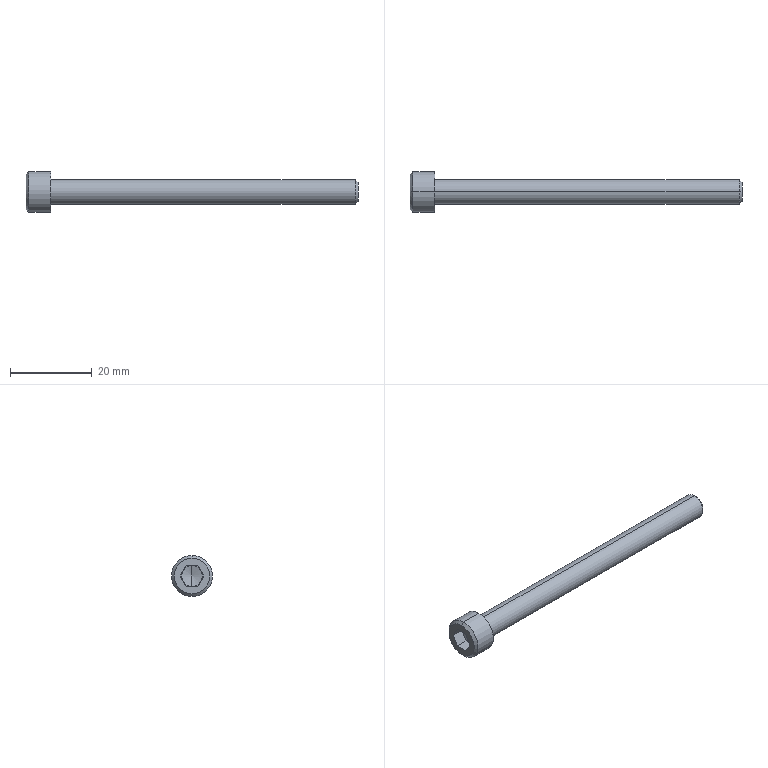Part | STEP file | 0245_307_SCB6-75 | 1 solid | 25 faces | box 81 x 10 x 10 mm | volume 2512 mm3 | plane 15 | cone 6 | cylinder 4 | commonest cylinder face diameters 6 x2 10 x2
STEP:
#1=CARTESIAN_POINT('',(0.,0.,0.));
#2=DIRECTION('',(0.,0.,1.));
#3=DIRECTION('',(1.,0.,0.));
#4=AXIS2_PLACEMENT_3D('',#1,#2,#3);
#5=CARTESIAN_POINT('',(75.,0.,-2.3));
#6=VERTEX_POINT('',#5);
#7=CARTESIAN_POINT('',(75.,0.,2.3));
#8=VERTEX_POINT('',#7);
#9=CARTESIAN_POINT('',(75.,0.,0.));
#10=DIRECTION('',(1.,0.,0.));
#11=DIRECTION('',(0.,0.,-1.));
#12=AXIS2_PLACEMENT_3D('',#9,#10,#11);
#13=CIRCLE('',#12,2.3);
#14=CARTESIAN_POINT('',(75.,0.,0.));
#15=DIRECTION('',(-1.,0.,0.));
#16=DIRECTION('',(0.,0.,1.));
#17=AXIS2_PLACEMENT_3D('',#14,#15,#16);
#18=CONICAL_SURFACE('',#17,2.3,0.7854);
#19=CARTESIAN_POINT('',(3.142,0.));
#20=DIRECTION('',(-1.,0.));
#21=VECTOR('',#20,1.);
#22=LINE('',#19,#21);
#23=(GEOMETRIC_REPRESENTATION_CONTEXT(2)PARAMETRIC_REPRESENTATION_CONTEXT()REPRESENTATION_CONTEXT('',''));
#24=DEFINITIONAL_REPRESENTATION('',(#22),#23);
#25=PCURVE('',#18,#24);
#26=CARTESIAN_POINT('',(75.,0.,0.));
#27=DIRECTION('',(1.,0.,0.));
#28=DIRECTION('',(0.,0.,-1.));
#29=AXIS2_PLACEMENT_3D('',#26,#27,#28);
#30=PLANE('',#29);
#31=CARTESIAN_POINT('',(0.,0.));
#32=DIRECTION('',(1.,0.));
#33=AXIS2_PLACEMENT_2D('',#31,#32);
#34=CIRCLE('',#33,2.3);
#35=(GEOMETRIC_REPRESENTATION_CONTEXT(2)PARAMETRIC_REPRESENTATION_CONTEXT()REPRESENTATION_CONTEXT('',''));
#36=DEFINITIONAL_REPRESENTATION('',(#34),#35);
#37=PCURVE('',#30,#36);
#38=SURFACE_CURVE('',#13,(#25,#37),.PCURVE_S1.);
#39=EDGE_CURVE('',#6,#8,#38,.T.);
#40=ORIENTED_EDGE('',*,*,#39,.F.);
#41=CARTESIAN_POINT('',(74.3,0.,-3.));
#42=VERTEX_POINT('',#41);
#43=CARTESIAN_POINT('',(75.,0.,-2.3));
#44=DIRECTION('',(-0.7071,0.,-0.7071));
#45=VECTOR('',#44,1.);
#46=LINE('',#43,#45);
#47=CARTESIAN_POINT('',(3.142,0.));
#48=DIRECTION('',(0.,1.));
#49=VECTOR('',#48,1.);
#50=LINE('',#47,#49);
#51=(GEOMETRIC_REPRESENTATION_CONTEXT(2)PARAMETRIC_REPRESENTATION_CONTEXT()REPRESENTATION_CONTEXT('',''));
#52=DEFINITIONAL_REPRESENTATION('',(#50),#51);
#53=PCURVE('',#18,#52);
#54=CARTESIAN_POINT('',(75.,0.,0.));
#55=DIRECTION('',(-1.,0.,0.));
#56=DIRECTION('',(0.,0.,1.));
#57=AXIS2_PLACEMENT_3D('',#54,#55,#56);
#58=CONICAL_SURFACE('',#57,2.3,0.7854);
#59=CARTESIAN_POINT('',(3.142,0.));
#60=DIRECTION('',(0.,1.));
#61=VECTOR('',#60,1.);
#62=LINE('',#59,#61);
#63=(GEOMETRIC_REPRESENTATION_CONTEXT(2)PARAMETRIC_REPRESENTATION_CONTEXT()REPRESENTATION_CONTEXT('',''));
#64=DEFINITIONAL_REPRESENTATION('',(#62),#63);
#65=PCURVE('',#58,#64);
#66=SURFACE_CURVE('',#46,(#53,#65),.PCURVE_S1.);
#67=EDGE_CURVE('',#6,#42,#66,.T.);
#68=ORIENTED_EDGE('',*,*,#67,.T.);
#69=CARTESIAN_POINT('',(74.3,0.,3.));
#70=VERTEX_POINT('',#69);
#71=CARTESIAN_POINT('',(74.3,0.,0.));
#72=DIRECTION('',(-1.,0.,0.));
#73=DIRECTION('',(0.,0.,-1.));
#74=AXIS2_PLACEMENT_3D('',#71,#72,#73);
#75=CIRCLE('',#74,3.);
#76=CARTESIAN_POINT('',(-3.142,0.7));
#77=DIRECTION('',(1.,0.));
#78=VECTOR('',#77,1.);
#79=LINE('',#76,#78);
#80=(GEOMETRIC_REPRESENTATION_CONTEXT(2)PARAMETRIC_REPRESENTATION_CONTEXT()REPRESENTATION_CONTEXT('',''));
#81=DEFINITIONAL_REPRESENTATION('',(#79),#80);
#82=PCURVE('',#18,#81);
#83=CARTESIAN_POINT('',(75.,0.,0.));
#84=DIRECTION('',(-1.,0.,0.));
#85=DIRECTION('',(0.,0.,1.));
#86=AXIS2_PLACEMENT_3D('',#83,#84,#85);
#87=CYLINDRICAL_SURFACE('',#86,3.);
#88=CARTESIAN_POINT('',(-3.142,0.7));
#89=DIRECTION('',(1.,0.));
#90=VECTOR('',#89,1.);
#91=LINE('',#88,#90);
#92=(GEOMETRIC_REPRESENTATION_CONTEXT(2)PARAMETRIC_REPRESENTATION_CONTEXT()REPRESENTATION_CONTEXT('',''));
#93=DEFINITIONAL_REPRESENTATION('',(#91),#92);
#94=PCURVE('',#87,#93);
#95=SURFACE_CURVE('',#75,(#82,#94),.PCURVE_S1.);
#96=EDGE_CURVE('',#70,#42,#95,.T.);
#97=ORIENTED_EDGE('',*,*,#96,.F.);
#98=CARTESIAN_POINT('',(75.,0.,2.3));
#99=DIRECTION('',(-0.7071,0.,0.7071));
#100=VECTOR('',#99,1.);
#101=LINE('',#98,#100);
#102=CARTESIAN_POINT('',(0.,0.));
#103=DIRECTION('',(0.,1.));
#104=VECTOR('',#103,1.);
#105=LINE('',#102,#104);
#106=(GEOMETRIC_REPRESENTATION_CONTEXT(2)PARAMETRIC_REPRESENTATION_CONTEXT()REPRESENTATION_CONTEXT('',''));
#107=DEFINITIONAL_REPRESENTATION('',(#105),#106);
#108=PCURVE('',#18,#107);
#109=CARTESIAN_POINT('',(6.283,0.));
#110=DIRECTION('',(0.,1.));
#111=VECTOR('',#110,1.);
#112=LINE('',#109,#111);
#113=(GEOMETRIC_REPRESENTATION_CONTEXT(2)PARAMETRIC_REPRESENTATION_CONTEXT()REPRESENTATION_CONTEXT('',''));
#114=DEFINITIONAL_REPRESENTATION('',(#112),#113);
#115=PCURVE('',#58,#114);
#116=SURFACE_CURVE('',#101,(#108,#115),.PCURVE_S1.);
#117=EDGE_CURVE('',#8,#70,#116,.T.);
#118=ORIENTED_EDGE('',*,*,#117,.F.);
#119=EDGE_LOOP('',(#40,#68,#97,#118));
#120=FACE_BOUND('',#119,.T.);
#121=ADVANCED_FACE('',(#120),#18,.T.);
#122=ORIENTED_EDGE('',*,*,#96,.T.);
#123=CARTESIAN_POINT('',(0.,0.,-3.));
#124=VERTEX_POINT('',#123);
#125=CARTESIAN_POINT('',(75.,0.,-3.));
#126=DIRECTION('',(-1.,0.,0.));
#127=VECTOR('',#126,1.);
#128=LINE('',#125,#127);
#129=CARTESIAN_POINT('',(3.142,0.));
#130=DIRECTION('',(0.,1.));
#131=VECTOR('',#130,1.);
#132=LINE('',#129,#131);
#133=(GEOMETRIC_REPRESENTATION_CONTEXT(2)PARAMETRIC_REPRESENTATION_CONTEXT()REPRESENTATION_CONTEXT('',''));
#134=DEFINITIONAL_REPRESENTATION('',(#132),#133);
#135=PCURVE('',#87,#134);
#136=CARTESIAN_POINT('',(75.,0.,0.));
#137=DIRECTION('',(-1.,0.,0.));
#138=DIRECTION('',(0.,0.,1.));
#139=AXIS2_PLACEMENT_3D('',#136,#137,#138);
#140=CYLINDRICAL_SURFACE('',#139,3.);
#141=CARTESIAN_POINT('',(3.142,0.));
#142=DIRECTION('',(0.,1.));
#143=VECTOR('',#142,1.);
#144=LINE('',#141,#143);
#145=(GEOMETRIC_REPRESENTATION_CONTEXT(2)PARAMETRIC_REPRESENTATION_CONTEXT()REPRESENTATION_CONTEXT('',''));
#146=DEFINITIONAL_REPRESENTATION('',(#144),#145);
#147=PCURVE('',#140,#146);
#148=SURFACE_CURVE('',#128,(#135,#147),.PCURVE_S1.);
#149=EDGE_CURVE('',#42,#124,#148,.T.);
#150=ORIENTED_EDGE('',*,*,#149,.T.);
#151=CARTESIAN_POINT('',(0.,0.,3.));
#152=VERTEX_POINT('',#151);
#153=CARTESIAN_POINT('',(0.,0.,0.));
#154=DIRECTION('',(1.,0.,0.));
#155=DIRECTION('',(0.,0.,-1.));
#156=AXIS2_PLACEMENT_3D('',#153,#154,#155);
#157=CIRCLE('',#156,3.);
#158=CARTESIAN_POINT('',(3.142,75.));
#159=DIRECTION('',(-1.,0.));
#160=VECTOR('',#159,1.);
#161=LINE('',#158,#160);
#162=(GEOMETRIC_REPRESENTATION_CONTEXT(2)PARAMETRIC_REPRESENTATION_CONTEXT()REPRESENTATION_CONTEXT('',''));
#163=DEFINITIONAL_REPRESENTATION('',(#161),#162);
#164=PCURVE('',#87,#163);
#165=CARTESIAN_POINT('',(0.,4.,0.));
#166=DIRECTION('',(1.,0.,0.));
#167=DIRECTION('',(0.,0.,-1.));
#168=AXIS2_PLACEMENT_3D('',#165,#166,#167);
#169=PLANE('',#168);
#170=CARTESIAN_POINT('',(0.,-4.));
#171=DIRECTION('',(1.,0.));
#172=AXIS2_PLACEMENT_2D('',#170,#171);
#173=CIRCLE('',#172,3.);
#174=(GEOMETRIC_REPRESENTATION_CONTEXT(2)PARAMETRIC_REPRESENTATION_CONTEXT()REPRESENTATION_CONTEXT('',''));
#175=DEFINITIONAL_REPRESENTATION('',(#173),#174);
#176=PCURVE('',#169,#175);
#177=SURFACE_CURVE('',#157,(#164,#176),.PCURVE_S1.);
#178=EDGE_CURVE('',#124,#152,#177,.T.);
#179=ORIENTED_EDGE('',*,*,#178,.T.);
#180=CARTESIAN_POINT('',(75.,0.,3.));
#181=DIRECTION('',(-1.,0.,0.));
#182=VECTOR('',#181,1.);
#183=LINE('',#180,#182);
#184=CARTESIAN_POINT('',(0.,0.));
#185=DIRECTION('',(0.,1.));
#186=VECTOR('',#185,1.);
#187=LINE('',#184,#186);
#188=(GEOMETRIC_REPRESENTATION_CONTEXT(2)PARAMETRIC_REPRESENTATION_CONTEXT()REPRESENTATION_CONTEXT('',''));
#189=DEFINITIONAL_REPRESENTATION('',(#187),#188);
#190=PCURVE('',#87,#189);
#191=CARTESIAN_POINT('',(6.283,0.));
#192=DIRECTION('',(0.,1.));
#193=VECTOR('',#192,1.);
#194=LINE('',#191,#193);
#195=(GEOMETRIC_REPRESENTATION_CONTEXT(2)PARAMETRIC_REPRESENTATION_CONTEXT()REPRESENTATION_CONTEXT('',''));
#196=DEFINITIONAL_REPRESENTATION('',(#194),#195);
#197=PCURVE('',#140,#196);
#198=SURFACE_CURVE('',#183,(#190,#197),.PCURVE_S1.);
#199=EDGE_CURVE('',#70,#152,#198,.T.);
#200=ORIENTED_EDGE('',*,*,#199,.F.);
#201=EDGE_LOOP('',(#122,#150,#179,#200));
#202=FACE_BOUND('',#201,.T.);
#203=ADVANCED_FACE('',(#202),#87,.T.);
#204=CARTESIAN_POINT('',(-5.333,0.,-5.));
#205=VERTEX_POINT('',#204);
#206=CARTESIAN_POINT('',(-5.333,0.,5.));
#207=VERTEX_POINT('',#206);
#208=CARTESIAN_POINT('',(-5.333,0.,0.));
#209=DIRECTION('',(1.,0.,0.));
#210=DIRECTION('',(0.,0.,-1.));
#211=AXIS2_PLACEMENT_3D('',#208,#209,#210);
#212=CIRCLE('',#211,5.);
#213=CARTESIAN_POINT('',(-2.667,0.,0.));
#214=DIRECTION('',(1.,0.,0.));
#215=DIRECTION('',(0.,0.,-1.));
#216=AXIS2_PLACEMENT_3D('',#213,#214,#215);
#217=CYLINDRICAL_SURFACE('',#216,5.);
#218=CARTESIAN_POINT('',(0.,-2.667));
#219=DIRECTION('',(1.,0.));
#220=VECTOR('',#219,1.);
#221=LINE('',#218,#220);
#222=(GEOMETRIC_REPRESENTATION_CONTEXT(2)PARAMETRIC_REPRESENTATION_CONTEXT()REPRESENTATION_CONTEXT('',''));
#223=DEFINITIONAL_REPRESENTATION('',(#221),#222);
#224=PCURVE('',#217,#223);
#225=CARTESIAN_POINT('',(-5.333,0.,0.));
#226=DIRECTION('',(1.,0.,0.));
#227=DIRECTION('',(0.,0.,-1.));
#228=AXIS2_PLACEMENT_3D('',#225,#226,#227);
#229=CONICAL_SURFACE('',#228,5.,0.7854);
#230=CARTESIAN_POINT('',(0.,0.));
#231=DIRECTION('',(1.,0.));
#232=VECTOR('',#231,1.);
#233=LINE('',#230,#232);
#234=(GEOMETRIC_REPRESENTATION_CONTEXT(2)PARAMETRIC_REPRESENTATION_CONTEXT()REPRESENTATION_CONTEXT('',''));
#235=DEFINITIONAL_REPRESENTATION('',(#233),#234);
#236=PCURVE('',#229,#235);
#237=SURFACE_CURVE('',#212,(#224,#236),.PCURVE_S1.);
#238=EDGE_CURVE('',#205,#207,#237,.T.);
#239=ORIENTED_EDGE('',*,*,#238,.T.);
#240=CARTESIAN_POINT('',(0.,0.,5.));
#241=VERTEX_POINT('',#240);
#242=CARTESIAN_POINT('',(-2.667,0.,5.));
#243=DIRECTION('',(1.,0.,0.));
#244=VECTOR('',#243,1.);
#245=LINE('',#242,#244);
#246=CARTESIAN_POINT('',(3.142,0.));
#247=DIRECTION('',(0.,1.));
#248=VECTOR('',#247,1.);
#249=LINE('',#246,#248);
#250=(GEOMETRIC_REPRESENTATION_CONTEXT(2)PARAMETRIC_REPRESENTATION_CONTEXT()REPRESENTATION_CONTEXT('',''));
#251=DEFINITIONAL_REPRESENTATION('',(#249),#250);
#252=PCURVE('',#217,#251);
#253=CARTESIAN_POINT('',(-2.667,0.,0.));
#254=DIRECTION('',(1.,0.,0.));
#255=DIRECTION('',(0.,0.,-1.));
#256=AXIS2_PLACEMENT_3D('',#253,#254,#255);
#257=CYLINDRICAL_SURFACE('',#256,5.);
#258=CARTESIAN_POINT('',(3.142,0.));
#259=DIRECTION('',(0.,1.));
#260=VECTOR('',#259,1.);
#261=LINE('',#258,#260);
#262=(GEOMETRIC_REPRESENTATION_CONTEXT(2)PARAMETRIC_REPRESENTATION_CONTEXT()REPRESENTATION_CONTEXT('',''));
#263=DEFINITIONAL_REPRESENTATION('',(#261),#262);
#264=PCURVE('',#257,#263);
#265=SURFACE_CURVE('',#245,(#252,#264),.PCURVE_S1.);
#266=EDGE_CURVE('',#207,#241,#265,.T.);
#267=ORIENTED_EDGE('',*,*,#266,.T.);
#268=CARTESIAN_POINT('',(0.,0.,-5.));
#269=VERTEX_POINT('',#268);
#270=CARTESIAN_POINT('',(0.,0.,0.));
#271=DIRECTION('',(1.,0.,0.));
#272=DIRECTION('',(0.,0.,-1.));
#273=AXIS2_PLACEMENT_3D('',#270,#271,#272);
#274=CIRCLE('',#273,5.);
#275=CARTESIAN_POINT('',(0.,2.667));
#276=DIRECTION('',(1.,0.));
#277=VECTOR('',#276,1.);
#278=LINE('',#275,#277);
#279=(GEOMETRIC_REPRESENTATION_CONTEXT(2)PARAMETRIC_REPRESENTATION_CONTEXT()REPRESENTATION_CONTEXT('',''));
#280=DEFINITIONAL_REPRESENTATION('',(#278),#279);
#281=PCURVE('',#217,#280);
#282=CARTESIAN_POINT('',(0.,-4.));
#283=DIRECTION('',(1.,0.));
#284=AXIS2_PLACEMENT_2D('',#282,#283);
#285=CIRCLE('',#284,5.);
#286=(GEOMETRIC_REPRESENTATION_CONTEXT(2)PARAMETRIC_REPRESENTATION_CONTEXT()REPRESENTATION_CONTEXT('',''));
#287=DEFINITIONAL_REPRESENTATION('',(#285),#286);
#288=PCURVE('',#169,#287);
#289=SURFACE_CURVE('',#274,(#281,#288),.PCURVE_S1.);
#290=EDGE_CURVE('',#269,#241,#289,.T.);
#291=ORIENTED_EDGE('',*,*,#290,.F.);
#292=CARTESIAN_POINT('',(-2.667,0.,-5.));
#293=DIRECTION('',(1.,0.,0.));
#294=VECTOR('',#293,1.);
#295=LINE('',#292,#294);
#296=CARTESIAN_POINT('',(0.,0.));
#297=DIRECTION('',(0.,1.));
#298=VECTOR('',#297,1.);
#299=LINE('',#296,#298);
#300=(GEOMETRIC_REPRESENTATION_CONTEXT(2)PARAMETRIC_REPRESENTATION_CONTEXT()REPRESENTATION_CONTEXT('',''));
#301=DEFINITIONAL_REPRESENTATION('',(#299),#300);
#302=PCURVE('',#217,#301);
#303=CARTESIAN_POINT('',(6.283,0.));
#304=DIRECTION('',(0.,1.));
#305=VECTOR('',#304,1.);
#306=LINE('',#303,#305);
#307=(GEOMETRIC_REPRESENTATION_CONTEXT(2)PARAMETRIC_REPRESENTATION_CONTEXT()REPRESENTATION_CONTEXT('',''));
#308=DEFINITIONAL_REPRESENTATION('',(#306),#307);
#309=PCURVE('',#257,#308);
#310=SURFACE_CURVE('',#295,(#302,#309),.PCURVE_S1.);
#311=EDGE_CURVE('',#205,#269,#310,.T.);
#312=ORIENTED_EDGE('',*,*,#311,.F.);
#313=EDGE_LOOP('',(#239,#267,#291,#312));
#314=FACE_BOUND('',#313,.T.);
#315=ADVANCED_FACE('',(#314),#217,.T.);
#316=CARTESIAN_POINT('',(-6.,0.,-4.333));
#317=VERTEX_POINT('',#316);
#318=CARTESIAN_POINT('',(-6.,0.,4.333));
#319=VERTEX_POINT('',#318);
#320=CARTESIAN_POINT('',(-6.,0.,0.));
#321=DIRECTION('',(1.,0.,0.));
#322=DIRECTION('',(0.,0.,-1.));
#323=AXIS2_PLACEMENT_3D('',#320,#321,#322);
#324=CIRCLE('',#323,4.333);
#325=CARTESIAN_POINT('',(0.,-0.6667));
#326=DIRECTION('',(1.,0.));
#327=VECTOR('',#326,1.);
#328=LINE('',#325,#327);
#329=(GEOMETRIC_REPRESENTATION_CONTEXT(2)PARAMETRIC_REPRESENTATION_CONTEXT()REPRESENTATION_CONTEXT('',''));
#330=DEFINITIONAL_REPRESENTATION('',(#328),#329);
#331=PCURVE('',#229,#330);
#332=CARTESIAN_POINT('',(-6.,2.167,0.));
#333=DIRECTION('',(-1.,0.,0.));
#334=DIRECTION('',(0.,0.,1.));
#335=AXIS2_PLACEMENT_3D('',#332,#333,#334);
#336=PLANE('',#335);
#337=CARTESIAN_POINT('',(-4.333,-2.167));
#338=CARTESIAN_POINT('',(-4.333,5.339));
#339=CARTESIAN_POINT('',(2.167,1.586));
#340=CARTESIAN_POINT('',(8.667,-2.167));
#341=CARTESIAN_POINT('',(2.167,-5.919));
#342=CARTESIAN_POINT('',(-4.333,-9.672));
#343=CARTESIAN_POINT('',(-4.333,-2.167));
#344=(BOUNDED_CURVE()B_SPLINE_CURVE(2,(#337,#338,#339,#340,#341,#342,#343),.UNSPECIFIED.,.T.,.F.)B_SPLINE_CURVE_WITH_KNOTS((1,2,2,2,2,1),(-2.094,0.,2.094,4.189,6.283,8.378),.UNSPECIFIED.)CURVE()GEOMETRIC_REPRESENTATION_ITEM()RATIONAL_B_SPLINE_CURVE((1.,0.5,1.,0.5,1.,0.5,1.))REPRESENTATION_ITEM(''));
#345=(GEOMETRIC_REPRESENTATION_CONTEXT(2)PARAMETRIC_REPRESENTATION_CONTEXT()REPRESENTATION_CONTEXT('',''));
#346=DEFINITIONAL_REPRESENTATION('',(#344),#345);
#347=PCURVE('',#336,#346);
#348=SURFACE_CURVE('',#324,(#331,#347),.PCURVE_S1.);
#349=EDGE_CURVE('',#317,#319,#348,.T.);
#350=ORIENTED_EDGE('',*,*,#349,.T.);
#351=CARTESIAN_POINT('',(-5.333,0.,5.));
#352=DIRECTION('',(0.7071,0.,0.7071));
#353=VECTOR('',#352,1.);
#354=LINE('',#351,#353);
#355=CARTESIAN_POINT('',(3.142,0.));
#356=DIRECTION('',(0.,1.));
#357=VECTOR('',#356,1.);
#358=LINE('',#355,#357);
#359=(GEOMETRIC_REPRESENTATION_CONTEXT(2)PARAMETRIC_REPRESENTATION_CONTEXT()REPRESENTATION_CONTEXT('',''));
#360=DEFINITIONAL_REPRESENTATION('',(#358),#359);
#361=PCURVE('',#229,#360);
#362=CARTESIAN_POINT('',(-5.333,0.,0.));
#363=DIRECTION('',(1.,0.,0.));
#364=DIRECTION('',(0.,0.,-1.));
#365=AXIS2_PLACEMENT_3D('',#362,#363,#364);
#366=CONICAL_SURFACE('',#365,5.,0.7854);
#367=CARTESIAN_POINT('',(3.142,0.));
#368=DIRECTION('',(0.,1.));
#369=VECTOR('',#368,1.);
#370=LINE('',#367,#369);
#371=(GEOMETRIC_REPRESENTATION_CONTEXT(2)PARAMETRIC_REPRESENTATION_CONTEXT()REPRESENTATION_CONTEXT('',''));
#372=DEFINITIONAL_REPRESENTATION('',(#370),#371);
#373=PCURVE('',#366,#372);
#374=SURFACE_CURVE('',#354,(#361,#373),.PCURVE_S1.);
#375=EDGE_CURVE('',#319,#207,#374,.T.);
#376=ORIENTED_EDGE('',*,*,#375,.T.);
#377=ORIENTED_EDGE('',*,*,#238,.F.);
#378=CARTESIAN_POINT('',(-5.333,0.,-5.));
#379=DIRECTION('',(0.7071,0.,-0.7071));
#380=VECTOR('',#379,1.);
#381=LINE('',#378,#380);
#382=CARTESIAN_POINT('',(0.,0.));
#383=DIRECTION('',(0.,1.));
#384=VECTOR('',#383,1.);
#385=LINE('',#382,#384);
#386=(GEOMETRIC_REPRESENTATION_CONTEXT(2)PARAMETRIC_REPRESENTATION_CONTEXT()REPRESENTATION_CONTEXT('',''));
#387=DEFINITIONAL_REPRESENTATION('',(#385),#386);
#388=PCURVE('',#229,#387);
#389=CARTESIAN_POINT('',(6.283,0.));
#390=DIRECTION('',(0.,1.));
#391=VECTOR('',#390,1.);
#392=LINE('',#389,#391);
#393=(GEOMETRIC_REPRESENTATION_CONTEXT(2)PARAMETRIC_REPRESENTATION_CONTEXT()REPRESENTATION_CONTEXT('',''));
#394=DEFINITIONAL_REPRESENTATION('',(#392),#393);
#395=PCURVE('',#366,#394);
#396=SURFACE_CURVE('',#381,(#388,#395),.PCURVE_S1.);
#397=EDGE_CURVE('',#317,#205,#396,.T.);
#398=ORIENTED_EDGE('',*,*,#397,.F.);
#399=EDGE_LOOP('',(#350,#376,#377,#398));
#400=FACE_BOUND('',#399,.T.);
#401=ADVANCED_FACE('',(#400),#229,.T.);
#402=CARTESIAN_POINT('',(-3.,-2.165,1.25));
#403=VERTEX_POINT('',#402);
#404=CARTESIAN_POINT('',(-3.,0.,2.5));
#405=VERTEX_POINT('',#404);
#406=CARTESIAN_POINT('',(-3.,0.,0.));
#407=DIRECTION('',(-1.,0.,0.));
#408=DIRECTION('',(0.,0.,1.));
#409=AXIS2_PLACEMENT_3D('',#406,#407,#408);
#410=CIRCLE('',#409,2.5);
#411=CARTESIAN_POINT('',(-3.,0.,0.));
#412=DIRECTION('',(-1.,0.,0.));
#413=DIRECTION('',(0.,0.,1.));
#414=AXIS2_PLACEMENT_3D('',#411,#412,#413);
#415=CONICAL_SURFACE('',#414,2.5,1.309);
#416=CARTESIAN_POINT('',(0.,0.));
#417=DIRECTION('',(1.,0.));
#418=VECTOR('',#417,1.);
#419=LINE('',#416,#418);
#420=(GEOMETRIC_REPRESENTATION_CONTEXT(2)PARAMETRIC_REPRESENTATION_CONTEXT()REPRESENTATION_CONTEXT('',''));
#421=DEFINITIONAL_REPRESENTATION('',(#419),#420);
#422=PCURVE('',#415,#421);
#423=CARTESIAN_POINT('',(-3.,0.,0.));
#424=DIRECTION('',(1.,0.,0.));
#425=DIRECTION('',(0.,0.,-1.));
#426=AXIS2_PLACEMENT_3D('',#423,#424,#425);
#427=PLANE('',#426);
#428=CARTESIAN_POINT('',(-2.5,0.));
#429=CARTESIAN_POINT('',(-2.5,4.33));
#430=CARTESIAN_POINT('',(1.25,2.165));
#431=CARTESIAN_POINT('',(5.,0.));
#432=CARTESIAN_POINT('',(1.25,-2.165));
#433=CARTESIAN_POINT('',(-2.5,-4.33));
#434=CARTESIAN_POINT('',(-2.5,0.));
#435=(BOUNDED_CURVE()B_SPLINE_CURVE(2,(#428,#429,#430,#431,#432,#433,#434),.UNSPECIFIED.,.T.,.F.)B_SPLINE_CURVE_WITH_KNOTS((1,2,2,2,2,1),(-2.094,0.,2.094,4.189,6.283,8.378),.UNSPECIFIED.)CURVE()GEOMETRIC_REPRESENTATION_ITEM()RATIONAL_B_SPLINE_CURVE((1.,0.5,1.,0.5,1.,0.5,1.))REPRESENTATION_ITEM(''));
#436=(GEOMETRIC_REPRESENTATION_CONTEXT(2)PARAMETRIC_REPRESENTATION_CONTEXT()REPRESENTATION_CONTEXT('',''));
#437=DEFINITIONAL_REPRESENTATION('',(#435),#436);
#438=PCURVE('',#427,#437);
#439=SURFACE_CURVE('',#410,(#422,#438),.PCURVE_S1.);
#440=EDGE_CURVE('',#403,#405,#439,.T.);
#441=ORIENTED_EDGE('',*,*,#440,.F.);
#442=CARTESIAN_POINT('',(-3.,-2.165,-1.25));
#443=VERTEX_POINT('',#442);
#444=CARTESIAN_POINT('',(-3.,0.,0.));
#445=DIRECTION('',(1.,0.,0.));
#446=DIRECTION('',(0.,0.,1.));
#447=AXIS2_PLACEMENT_3D('',#444,#445,#446);
#448=CIRCLE('',#447,2.5);
#449=CARTESIAN_POINT('',(6.283,0.));
#450=DIRECTION('',(-1.,0.));
#451=VECTOR('',#450,1.);
#452=LINE('',#449,#451);
#453=(GEOMETRIC_REPRESENTATION_CONTEXT(2)PARAMETRIC_REPRESENTATION_CONTEXT()REPRESENTATION_CONTEXT('',''));
#454=DEFINITIONAL_REPRESENTATION('',(#452),#453);
#455=PCURVE('',#415,#454);
#456=CARTESIAN_POINT('',(-3.,0.,0.));
#457=DIRECTION('',(1.,0.,0.));
#458=DIRECTION('',(0.,0.,-1.));
#459=AXIS2_PLACEMENT_3D('',#456,#457,#458);
#460=PLANE('',#459);
#461=CARTESIAN_POINT('',(0.,0.));
#462=DIRECTION('',(-1.,0.));
#463=AXIS2_PLACEMENT_2D('',#461,#462);
#464=CIRCLE('',#463,2.5);
#465=(GEOMETRIC_REPRESENTATION_CONTEXT(2)PARAMETRIC_REPRESENTATION_CONTEXT()REPRESENTATION_CONTEXT('',''));
#466=DEFINITIONAL_REPRESENTATION('',(#464),#465);
#467=PCURVE('',#460,#466);
#468=SURFACE_CURVE('',#448,(#455,#467),.PCURVE_S1.);
#469=EDGE_CURVE('',#403,#443,#468,.T.);
#470=ORIENTED_EDGE('',*,*,#469,.T.);
#471=CARTESIAN_POINT('',(-3.,0.,-2.5));
#472=VERTEX_POINT('',#471);
#473=CARTESIAN_POINT('',(-3.,0.,0.));
#474=DIRECTION('',(1.,0.,0.));
#475=DIRECTION('',(0.,0.,1.));
#476=AXIS2_PLACEMENT_3D('',#473,#474,#475);
#477=CIRCLE('',#476,2.5);
#478=CARTESIAN_POINT('',(6.283,0.));
#479=DIRECTION('',(-1.,0.));
#480=VECTOR('',#479,1.);
#481=LINE('',#478,#480);
#482=(GEOMETRIC_REPRESENTATION_CONTEXT(2)PARAMETRIC_REPRESENTATION_CONTEXT()REPRESENTATION_CONTEXT('',''));
#483=DEFINITIONAL_REPRESENTATION('',(#481),#482);
#484=PCURVE('',#415,#483);
#485=CARTESIAN_POINT('',(-3.,0.,0.));
#486=DIRECTION('',(1.,0.,0.));
#487=DIRECTION('',(0.,0.,-1.));
#488=AXIS2_PLACEMENT_3D('',#485,#486,#487);
#489=PLANE('',#488);
#490=CARTESIAN_POINT('',(0.,0.));
#491=DIRECTION('',(-1.,0.));
#492=AXIS2_PLACEMENT_2D('',#490,#491);
#493=CIRCLE('',#492,2.5);
#494=(GEOMETRIC_REPRESENTATION_CONTEXT(2)PARAMETRIC_REPRESENTATION_CONTEXT()REPRESENTATION_CONTEXT('',''));
#495=DEFINITIONAL_REPRESENTATION('',(#493),#494);
#496=PCURVE('',#489,#495);
#497=SURFACE_CURVE('',#477,(#484,#496),.PCURVE_S1.);
#498=EDGE_CURVE('',#443,#472,#497,.T.);
#499=ORIENTED_EDGE('',*,*,#498,.T.);
#500=CARTESIAN_POINT('',(-2.33,0.,0.));
#501=VERTEX_POINT('',#500);
#502=CARTESIAN_POINT('',(-3.,0.,-2.5));
#503=DIRECTION('',(-0.2588,0.,-0.9659));
#504=VECTOR('',#503,1.);
#505=LINE('',#502,#504);
#506=CARTESIAN_POINT('',(3.142,0.));
#507=DIRECTION('',(0.,1.));
#508=VECTOR('',#507,1.);
#509=LINE('',#506,#508);
#510=(GEOMETRIC_REPRESENTATION_CONTEXT(2)PARAMETRIC_REPRESENTATION_CONTEXT()REPRESENTATION_CONTEXT('',''));
#511=DEFINITIONAL_REPRESENTATION('',(#509),#510);
#512=PCURVE('',#415,#511);
#513=CARTESIAN_POINT('',(-3.,0.,0.));
#514=DIRECTION('',(-1.,0.,0.));
#515=DIRECTION('',(0.,0.,1.));
#516=AXIS2_PLACEMENT_3D('',#513,#514,#515);
#517=CONICAL_SURFACE('',#516,2.5,1.309);
#518=CARTESIAN_POINT('',(3.142,0.));
#519=DIRECTION('',(0.,1.));
#520=VECTOR('',#519,1.);
#521=LINE('',#518,#520);
#522=(GEOMETRIC_REPRESENTATION_CONTEXT(2)PARAMETRIC_REPRESENTATION_CONTEXT()REPRESENTATION_CONTEXT('',''));
#523=DEFINITIONAL_REPRESENTATION('',(#521),#522);
#524=PCURVE('',#517,#523);
#525=SURFACE_CURVE('',#505,(#512,#524),.PCURVE_S1.);
#526=EDGE_CURVE('',#501,#472,#525,.T.);
#527=ORIENTED_EDGE('',*,*,#526,.F.);
#528=CARTESIAN_POINT('',(-3.,0.,2.5));
#529=DIRECTION('',(-0.2588,0.,0.9659));
#530=VECTOR('',#529,1.);
#531=LINE('',#528,#530);
#532=CARTESIAN_POINT('',(6.283,0.));
#533=DIRECTION('',(0.,1.));
#534=VECTOR('',#533,1.);
#535=LINE('',#532,#534);
#536=(GEOMETRIC_REPRESENTATION_CONTEXT(2)PARAMETRIC_REPRESENTATION_CONTEXT()REPRESENTATION_CONTEXT('',''));
#537=DEFINITIONAL_REPRESENTATION('',(#535),#536);
#538=PCURVE('',#415,#537);
#539=CARTESIAN_POINT('',(0.,0.));
#540=DIRECTION('',(0.,1.));
#541=VECTOR('',#540,1.);
#542=LINE('',#539,#541);
#543=(GEOMETRIC_REPRESENTATION_CONTEXT(2)PARAMETRIC_REPRESENTATION_CONTEXT()REPRESENTATION_CONTEXT('',''));
#544=DEFINITIONAL_REPRESENTATION('',(#542),#543);
#545=PCURVE('',#517,#544);
#546=SURFACE_CURVE('',#531,(#538,#545),.PCURVE_S1.);
#547=EDGE_CURVE('',#501,#405,#546,.T.);
#548=ORIENTED_EDGE('',*,*,#547,.T.);
#549=EDGE_LOOP('',(#441,#470,#499,#527,#548));
#550=FACE_BOUND('',#549,.F.);
#551=ADVANCED_FACE('',(#550),#415,.F.);
#552=ORIENTED_EDGE('',*,*,#290,.T.);
#553=CARTESIAN_POINT('',(0.,0.,0.));
#554=DIRECTION('',(1.,0.,0.));
#555=DIRECTION('',(0.,0.,-1.));
#556=AXIS2_PLACEMENT_3D('',#553,#554,#555);
#557=CIRCLE('',#556,5.);
#558=CARTESIAN_POINT('',(0.,-4.));
#559=DIRECTION('',(1.,0.));
#560=AXIS2_PLACEMENT_2D('',#558,#559);
#561=CIRCLE('',#560,5.);
#562=(GEOMETRIC_REPRESENTATION_CONTEXT(2)PARAMETRIC_REPRESENTATION_CONTEXT()REPRESENTATION_CONTEXT('',''));
#563=DEFINITIONAL_REPRESENTATION('',(#561),#562);
#564=PCURVE('',#169,#563);
#565=CARTESIAN_POINT('',(0.,2.667));
#566=DIRECTION('',(1.,0.));
#567=VECTOR('',#566,1.);
#568=LINE('',#565,#567);
#569=(GEOMETRIC_REPRESENTATION_CONTEXT(2)PARAMETRIC_REPRESENTATION_CONTEXT()REPRESENTATION_CONTEXT('',''));
#570=DEFINITIONAL_REPRESENTATION('',(#568),#569);
#571=PCURVE('',#257,#570);
#572=SURFACE_CURVE('',#557,(#564,#571),.PCURVE_S1.);
#573=EDGE_CURVE('',#241,#269,#572,.T.);
#574=ORIENTED_EDGE('',*,*,#573,.T.);
#575=EDGE_LOOP('',(#552,#574));
#576=FACE_BOUND('',#575,.T.);
#577=CARTESIAN_POINT('',(0.,0.,0.));
#578=DIRECTION('',(1.,0.,0.));
#579=DIRECTION('',(0.,0.,-1.));
#580=AXIS2_PLACEMENT_3D('',#577,#578,#579);
#581=CIRCLE('',#580,3.);
#582=CARTESIAN_POINT('',(0.,-4.));
#583=DIRECTION('',(1.,0.));
#584=AXIS2_PLACEMENT_2D('',#582,#583);
#585=CIRCLE('',#584,3.);
#586=(GEOMETRIC_REPRESENTATION_CONTEXT(2)PARAMETRIC_REPRESENTATION_CONTEXT()REPRESENTATION_CONTEXT('',''));
#587=DEFINITIONAL_REPRESENTATION('',(#585),#586);
#588=PCURVE('',#169,#587);
#589=CARTESIAN_POINT('',(9.425,75.));
#590=DIRECTION('',(-1.,0.));
#591=VECTOR('',#590,1.);
#592=LINE('',#589,#591);
#593=(GEOMETRIC_REPRESENTATION_CONTEXT(2)PARAMETRIC_REPRESENTATION_CONTEXT()REPRESENTATION_CONTEXT('',''));
#594=DEFINITIONAL_REPRESENTATION('',(#592),#593);
#595=PCURVE('',#140,#594);
#596=SURFACE_CURVE('',#581,(#588,#595),.PCURVE_S1.);
#597=EDGE_CURVE('',#152,#124,#596,.T.);
#598=ORIENTED_EDGE('',*,*,#597,.F.);
#599=ORIENTED_EDGE('',*,*,#178,.F.);
#600=EDGE_LOOP('',(#598,#599));
#601=FACE_BOUND('',#600,.T.);
#602=ADVANCED_FACE('',(#576,#601),#169,.T.);
#603=ORIENTED_EDGE('',*,*,#266,.F.);
#604=CARTESIAN_POINT('',(-5.333,0.,0.));
#605=DIRECTION('',(1.,0.,0.));
#606=DIRECTION('',(0.,0.,-1.));
#607=AXIS2_PLACEMENT_3D('',#604,#605,#606);
#608=CIRCLE('',#607,5.);
#609=CARTESIAN_POINT('',(0.,-2.667));
#610=DIRECTION('',(1.,0.));
#611=VECTOR('',#610,1.);
#612=LINE('',#609,#611);
#613=(GEOMETRIC_REPRESENTATION_CONTEXT(2)PARAMETRIC_REPRESENTATION_CONTEXT()REPRESENTATION_CONTEXT('',''));
#614=DEFINITIONAL_REPRESENTATION('',(#612),#613);
#615=PCURVE('',#257,#614);
#616=CARTESIAN_POINT('',(0.,0.));
#617=DIRECTION('',(1.,0.));
#618=VECTOR('',#617,1.);
#619=LINE('',#616,#618);
#620=(GEOMETRIC_REPRESENTATION_CONTEXT(2)PARAMETRIC_REPRESENTATION_CONTEXT()REPRESENTATION_CONTEXT('',''));
#621=DEFINITIONAL_REPRESENTATION('',(#619),#620);
#622=PCURVE('',#366,#621);
#623=SURFACE_CURVE('',#608,(#615,#622),.PCURVE_S1.);
#624=EDGE_CURVE('',#207,#205,#623,.T.);
#625=ORIENTED_EDGE('',*,*,#624,.T.);
#626=ORIENTED_EDGE('',*,*,#311,.T.);
#627=ORIENTED_EDGE('',*,*,#573,.F.);
#628=EDGE_LOOP('',(#603,#625,#626,#627));
#629=FACE_BOUND('',#628,.T.);
#630=ADVANCED_FACE('',(#629),#257,.T.);
#631=ORIENTED_EDGE('',*,*,#375,.F.);
#632=CARTESIAN_POINT('',(-6.,0.,0.));
#633=DIRECTION('',(1.,0.,0.));
#634=DIRECTION('',(0.,0.,-1.));
#635=AXIS2_PLACEMENT_3D('',#632,#633,#634);
#636=CIRCLE('',#635,4.333);
#637=CARTESIAN_POINT('',(0.,-0.6667));
#638=DIRECTION('',(1.,0.));
#639=VECTOR('',#638,1.);
#640=LINE('',#637,#639);
#641=(GEOMETRIC_REPRESENTATION_CONTEXT(2)PARAMETRIC_REPRESENTATION_CONTEXT()REPRESENTATION_CONTEXT('',''));
#642=DEFINITIONAL_REPRESENTATION('',(#640),#641);
#643=PCURVE('',#366,#642);
#644=CARTESIAN_POINT('',(-4.333,-2.167));
#645=CARTESIAN_POINT('',(-4.333,5.339));
#646=CARTESIAN_POINT('',(2.167,1.586));
#647=CARTESIAN_POINT('',(8.667,-2.167));
#648=CARTESIAN_POINT('',(2.167,-5.919));
#649=CARTESIAN_POINT('',(-4.333,-9.672));
#650=CARTESIAN_POINT('',(-4.333,-2.167));
#651=(BOUNDED_CURVE()B_SPLINE_CURVE(2,(#644,#645,#646,#647,#648,#649,#650),.UNSPECIFIED.,.T.,.F.)B_SPLINE_CURVE_WITH_KNOTS((1,2,2,2,2,1),(-2.094,0.,2.094,4.189,6.283,8.378),.UNSPECIFIED.)CURVE()GEOMETRIC_REPRESENTATION_ITEM()RATIONAL_B_SPLINE_CURVE((1.,0.5,1.,0.5,1.,0.5,1.))REPRESENTATION_ITEM(''));
#652=(GEOMETRIC_REPRESENTATION_CONTEXT(2)PARAMETRIC_REPRESENTATION_CONTEXT()REPRESENTATION_CONTEXT('',''));
#653=DEFINITIONAL_REPRESENTATION('',(#651),#652);
#654=PCURVE('',#336,#653);
#655=SURFACE_CURVE('',#636,(#643,#654),.PCURVE_S1.);
#656=EDGE_CURVE('',#319,#317,#655,.T.);
#657=ORIENTED_EDGE('',*,*,#656,.T.);
#658=ORIENTED_EDGE('',*,*,#397,.T.);
#659=ORIENTED_EDGE('',*,*,#624,.F.);
#660=EDGE_LOOP('',(#631,#657,#658,#659));
#661=FACE_BOUND('',#660,.T.);
#662=ADVANCED_FACE('',(#661),#366,.T.);
#663=CARTESIAN_POINT('',(-6.,1.443,-2.5));
#664=VERTEX_POINT('',#663);
#665=CARTESIAN_POINT('',(-6.,2.887,0.));
#666=VERTEX_POINT('',#665);
#667=CARTESIAN_POINT('',(-6.,1.443,-2.5));
#668=DIRECTION('',(0.,0.5,0.866));
#669=VECTOR('',#668,1.);
#670=LINE('',#667,#669);
#671=CARTESIAN_POINT('',(-2.5,-0.7233));
#672=DIRECTION('',(0.866,0.5));
#673=VECTOR('',#672,1.);
#674=LINE('',#671,#673);
#675=(GEOMETRIC_REPRESENTATION_CONTEXT(2)PARAMETRIC_REPRESENTATION_CONTEXT()REPRESENTATION_CONTEXT('',''));
#676=DEFINITIONAL_REPRESENTATION('',(#674),#675);
#677=PCURVE('',#336,#676);
#678=CARTESIAN_POINT('',(-6.,2.887,0.));
#679=DIRECTION('',(0.,0.866,-0.5));
#680=DIRECTION('',(0.,0.5,0.866));
#681=AXIS2_PLACEMENT_3D('',#678,#679,#680);
#682=PLANE('',#681);
#683=CARTESIAN_POINT('',(-2.887,0.));
#684=DIRECTION('',(1.,0.));
#685=VECTOR('',#684,1.);
#686=LINE('',#683,#685);
#687=(GEOMETRIC_REPRESENTATION_CONTEXT(2)PARAMETRIC_REPRESENTATION_CONTEXT()REPRESENTATION_CONTEXT('',''));
#688=DEFINITIONAL_REPRESENTATION('',(#686),#687);
#689=PCURVE('',#682,#688);
#690=SURFACE_CURVE('',#670,(#677,#689),.PCURVE_S1.);
#691=EDGE_CURVE('',#664,#666,#690,.T.);
#692=ORIENTED_EDGE('',*,*,#691,.T.);
#693=CARTESIAN_POINT('',(-6.,1.443,2.5));
#694=VERTEX_POINT('',#693);
#695=CARTESIAN_POINT('',(-6.,2.887,0.));
#696=DIRECTION('',(0.,-0.5,0.866));
#697=VECTOR('',#696,1.);
#698=LINE('',#695,#697);
#699=CARTESIAN_POINT('',(0.,0.7201));
#700=DIRECTION('',(0.866,-0.5));
#701=VECTOR('',#700,1.);
#702=LINE('',#699,#701);
#703=(GEOMETRIC_REPRESENTATION_CONTEXT(2)PARAMETRIC_REPRESENTATION_CONTEXT()REPRESENTATION_CONTEXT('',''));
#704=DEFINITIONAL_REPRESENTATION('',(#702),#703);
#705=PCURVE('',#336,#704);
#706=CARTESIAN_POINT('',(-6.,1.443,2.5));
#707=DIRECTION('',(0.,0.866,0.5));
#708=DIRECTION('',(0.,-0.5,0.866));
#709=AXIS2_PLACEMENT_3D('',#706,#707,#708);
#710=PLANE('',#709);
#711=CARTESIAN_POINT('',(-2.887,0.));
#712=DIRECTION('',(1.,0.));
#713=VECTOR('',#712,1.);
#714=LINE('',#711,#713);
#715=(GEOMETRIC_REPRESENTATION_CONTEXT(2)PARAMETRIC_REPRESENTATION_CONTEXT()REPRESENTATION_CONTEXT('',''));
#716=DEFINITIONAL_REPRESENTATION('',(#714),#715);
#717=PCURVE('',#710,#716);
#718=SURFACE_CURVE('',#698,(#705,#717),.PCURVE_S1.);
#719=EDGE_CURVE('',#666,#694,#718,.T.);
#720=ORIENTED_EDGE('',*,*,#719,.T.);
#721=CARTESIAN_POINT('',(-6.,-1.443,2.5));
#722=VERTEX_POINT('',#721);
#723=CARTESIAN_POINT('',(-6.,2.167,2.5));
#724=DIRECTION('',(0.,-1.,0.));
#725=VECTOR('',#724,1.);
#726=LINE('',#723,#725);
#727=CARTESIAN_POINT('',(2.5,0.));
#728=DIRECTION('',(0.,-1.));
#729=VECTOR('',#728,1.);
#730=LINE('',#727,#729);
#731=(GEOMETRIC_REPRESENTATION_CONTEXT(2)PARAMETRIC_REPRESENTATION_CONTEXT()REPRESENTATION_CONTEXT('',''));
#732=DEFINITIONAL_REPRESENTATION('',(#730),#731);
#733=PCURVE('',#336,#732);
#734=CARTESIAN_POINT('',(-6.,-1.443,2.5));
#735=DIRECTION('',(0.,0.,1.));
#736=DIRECTION('',(1.,0.,0.));
#737=AXIS2_PLACEMENT_3D('',#734,#735,#736);
#738=PLANE('',#737);
#739=CARTESIAN_POINT('',(0.,3.61));
#740=DIRECTION('',(0.,-1.));
#741=VECTOR('',#740,1.);
#742=LINE('',#739,#741);
#743=(GEOMETRIC_REPRESENTATION_CONTEXT(2)PARAMETRIC_REPRESENTATION_CONTEXT()REPRESENTATION_CONTEXT('',''));
#744=DEFINITIONAL_REPRESENTATION('',(#742),#743);
#745=PCURVE('',#738,#744);
#746=SURFACE_CURVE('',#726,(#733,#745),.PCURVE_S1.);
#747=EDGE_CURVE('',#694,#722,#746,.T.);
#748=ORIENTED_EDGE('',*,*,#747,.T.);
#749=CARTESIAN_POINT('',(-6.,-2.887,0.));
#750=VERTEX_POINT('',#749);
#751=CARTESIAN_POINT('',(-6.,-1.443,2.5));
#752=DIRECTION('',(0.,-0.5,-0.866));
#753=VECTOR('',#752,1.);
#754=LINE('',#751,#753);
#755=CARTESIAN_POINT('',(2.5,-3.61));
#756=DIRECTION('',(-0.866,-0.5));
#757=VECTOR('',#756,1.);
#758=LINE('',#755,#757);
#759=(GEOMETRIC_REPRESENTATION_CONTEXT(2)PARAMETRIC_REPRESENTATION_CONTEXT()REPRESENTATION_CONTEXT('',''));
#760=DEFINITIONAL_REPRESENTATION('',(#758),#759);
#761=PCURVE('',#336,#760);
#762=CARTESIAN_POINT('',(-6.,-2.887,0.));
#763=DIRECTION('',(0.,-0.866,0.5));
#764=DIRECTION('',(0.,-0.5,-0.866));
#765=AXIS2_PLACEMENT_3D('',#762,#763,#764);
#766=PLANE('',#765);
#767=CARTESIAN_POINT('',(-2.887,0.));
#768=DIRECTION('',(1.,0.));
#769=VECTOR('',#768,1.);
#770=LINE('',#767,#769);
#771=(GEOMETRIC_REPRESENTATION_CONTEXT(2)PARAMETRIC_REPRESENTATION_CONTEXT()REPRESENTATION_CONTEXT('',''));
#772=DEFINITIONAL_REPRESENTATION('',(#770),#771);
#773=PCURVE('',#766,#772);
#774=SURFACE_CURVE('',#754,(#761,#773),.PCURVE_S1.);
#775=EDGE_CURVE('',#722,#750,#774,.T.);
#776=ORIENTED_EDGE('',*,*,#775,.T.);
#777=CARTESIAN_POINT('',(-6.,-1.443,-2.5));
#778=VERTEX_POINT('',#777);
#779=CARTESIAN_POINT('',(-6.,-2.887,0.));
#780=DIRECTION('',(0.,0.5,-0.866));
#781=VECTOR('',#780,1.);
#782=LINE('',#779,#781);
#783=CARTESIAN_POINT('',(0.,-5.053));
#784=DIRECTION('',(-0.866,0.5));
#785=VECTOR('',#784,1.);
#786=LINE('',#783,#785);
#787=(GEOMETRIC_REPRESENTATION_CONTEXT(2)PARAMETRIC_REPRESENTATION_CONTEXT()REPRESENTATION_CONTEXT('',''));
#788=DEFINITIONAL_REPRESENTATION('',(#786),#787);
#789=PCURVE('',#336,#788);
#790=CARTESIAN_POINT('',(-6.,-1.443,-2.5));
#791=DIRECTION('',(0.,-0.866,-0.5));
#792=DIRECTION('',(0.,0.5,-0.866));
#793=AXIS2_PLACEMENT_3D('',#790,#791,#792);
#794=PLANE('',#793);
#795=CARTESIAN_POINT('',(-2.887,0.));
#796=DIRECTION('',(1.,0.));
#797=VECTOR('',#796,1.);
#798=LINE('',#795,#797);
#799=(GEOMETRIC_REPRESENTATION_CONTEXT(2)PARAMETRIC_REPRESENTATION_CONTEXT()REPRESENTATION_CONTEXT('',''));
#800=DEFINITIONAL_REPRESENTATION('',(#798),#799);
#801=PCURVE('',#794,#800);
#802=SURFACE_CURVE('',#782,(#789,#801),.PCURVE_S1.);
#803=EDGE_CURVE('',#750,#778,#802,.T.);
#804=ORIENTED_EDGE('',*,*,#803,.T.);
#805=CARTESIAN_POINT('',(-6.,2.167,-2.5));
#806=DIRECTION('',(0.,1.,0.));
#807=VECTOR('',#806,1.);
#808=LINE('',#805,#807);
#809=CARTESIAN_POINT('',(-2.5,0.));
#810=DIRECTION('',(0.,1.));
#811=VECTOR('',#810,1.);
#812=LINE('',#809,#811);
#813=(GEOMETRIC_REPRESENTATION_CONTEXT(2)PARAMETRIC_REPRESENTATION_CONTEXT()REPRESENTATION_CONTEXT('',''));
#814=DEFINITIONAL_REPRESENTATION('',(#812),#813);
#815=PCURVE('',#336,#814);
#816=CARTESIAN_POINT('',(-6.,1.443,-2.5));
#817=DIRECTION('',(0.,0.,-1.));
#818=DIRECTION('',(-1.,0.,0.));
#819=AXIS2_PLACEMENT_3D('',#816,#817,#818);
#820=PLANE('',#819);
#821=CARTESIAN_POINT('',(0.,0.7233));
#822=DIRECTION('',(0.,1.));
#823=VECTOR('',#822,1.);
#824=LINE('',#821,#823);
#825=(GEOMETRIC_REPRESENTATION_CONTEXT(2)PARAMETRIC_REPRESENTATION_CONTEXT()REPRESENTATION_CONTEXT('',''));
#826=DEFINITIONAL_REPRESENTATION('',(#824),#825);
#827=PCURVE('',#820,#826);
#828=SURFACE_CURVE('',#808,(#815,#827),.PCURVE_S1.);
#829=EDGE_CURVE('',#778,#664,#828,.T.);
#830=ORIENTED_EDGE('',*,*,#829,.T.);
#831=EDGE_LOOP('',(#692,#720,#748,#776,#804,#830));
#832=FACE_BOUND('',#831,.T.);
#833=ORIENTED_EDGE('',*,*,#349,.F.);
#834=ORIENTED_EDGE('',*,*,#656,.F.);
#835=EDGE_LOOP('',(#833,#834));
#836=FACE_BOUND('',#835,.T.);
#837=ADVANCED_FACE('',(#832,#836),#336,.T.);
#838=CARTESIAN_POINT('',(-3.,1.443,2.5));
#839=VERTEX_POINT('',#838);
#840=CARTESIAN_POINT('',(-6.,1.443,2.5));
#841=DIRECTION('',(1.,0.,0.));
#842=VECTOR('',#841,1.);
#843=LINE('',#840,#842);
#844=CARTESIAN_POINT('',(0.,0.));
#845=DIRECTION('',(0.,1.));
#846=VECTOR('',#845,1.);
#847=LINE('',#844,#846);
#848=(GEOMETRIC_REPRESENTATION_CONTEXT(2)PARAMETRIC_REPRESENTATION_CONTEXT()REPRESENTATION_CONTEXT('',''));
#849=DEFINITIONAL_REPRESENTATION('',(#847),#848);
#850=PCURVE('',#710,#849);
#851=CARTESIAN_POINT('',(0.,2.887));
#852=DIRECTION('',(1.,0.));
#853=VECTOR('',#852,1.);
#854=LINE('',#851,#853);
#855=(GEOMETRIC_REPRESENTATION_CONTEXT(2)PARAMETRIC_REPRESENTATION_CONTEXT()REPRESENTATION_CONTEXT('',''));
#856=DEFINITIONAL_REPRESENTATION('',(#854),#855);
#857=PCURVE('',#738,#856);
#858=SURFACE_CURVE('',#843,(#850,#857),.PCURVE_S1.);
#859=EDGE_CURVE('',#694,#839,#858,.T.);
#860=ORIENTED_EDGE('',*,*,#859,.F.);
#861=ORIENTED_EDGE('',*,*,#719,.F.);
#862=CARTESIAN_POINT('',(-3.,2.887,0.));
#863=VERTEX_POINT('',#862);
#864=CARTESIAN_POINT('',(-6.,2.887,0.));
#865=DIRECTION('',(-1.,0.,0.));
#866=VECTOR('',#865,1.);
#867=LINE('',#864,#866);
#868=CARTESIAN_POINT('',(-2.887,0.));
#869=DIRECTION('',(0.,-1.));
#870=VECTOR('',#869,1.);
#871=LINE('',#868,#870);
#872=(GEOMETRIC_REPRESENTATION_CONTEXT(2)PARAMETRIC_REPRESENTATION_CONTEXT()REPRESENTATION_CONTEXT('',''));
#873=DEFINITIONAL_REPRESENTATION('',(#871),#872);
#874=PCURVE('',#710,#873);
#875=CARTESIAN_POINT('',(0.,0.));
#876=DIRECTION('',(0.,-1.));
#877=VECTOR('',#876,1.);
#878=LINE('',#875,#877);
#879=(GEOMETRIC_REPRESENTATION_CONTEXT(2)PARAMETRIC_REPRESENTATION_CONTEXT()REPRESENTATION_CONTEXT('',''));
#880=DEFINITIONAL_REPRESENTATION('',(#878),#879);
#881=PCURVE('',#682,#880);
#882=SURFACE_CURVE('',#867,(#874,#881),.PCURVE_S1.);
#883=EDGE_CURVE('',#863,#666,#882,.T.);
#884=ORIENTED_EDGE('',*,*,#883,.F.);
#885=CARTESIAN_POINT('',(-3.,2.165,1.25));
#886=VERTEX_POINT('',#885);
#887=CARTESIAN_POINT('',(-3.,2.887,0.));
#888=DIRECTION('',(0.,-0.5,0.866));
#889=VECTOR('',#888,1.);
#890=LINE('',#887,#889);
#891=CARTESIAN_POINT('',(-2.887,3.));
#892=DIRECTION('',(1.,0.));
#893=VECTOR('',#892,1.);
#894=LINE('',#891,#893);
#895=(GEOMETRIC_REPRESENTATION_CONTEXT(2)PARAMETRIC_REPRESENTATION_CONTEXT()REPRESENTATION_CONTEXT('',''));
#896=DEFINITIONAL_REPRESENTATION('',(#894),#895);
#897=PCURVE('',#710,#896);
#898=CARTESIAN_POINT('',(-3.,0.,0.));
#899=DIRECTION('',(1.,0.,0.));
#900=DIRECTION('',(0.,0.,-1.));
#901=AXIS2_PLACEMENT_3D('',#898,#899,#900);
#902=PLANE('',#901);
#903=CARTESIAN_POINT('',(0.,2.887));
#904=DIRECTION('',(-0.866,-0.5));
#905=VECTOR('',#904,1.);
#906=LINE('',#903,#905);
#907=(GEOMETRIC_REPRESENTATION_CONTEXT(2)PARAMETRIC_REPRESENTATION_CONTEXT()REPRESENTATION_CONTEXT('',''));
#908=DEFINITIONAL_REPRESENTATION('',(#906),#907);
#909=PCURVE('',#902,#908);
#910=SURFACE_CURVE('',#890,(#897,#909),.PCURVE_S1.);
#911=EDGE_CURVE('',#863,#886,#910,.T.);
#912=ORIENTED_EDGE('',*,*,#911,.T.);
#913=CARTESIAN_POINT('',(-3.,2.165,1.25));
#914=DIRECTION('',(0.,-0.5,0.866));
#915=VECTOR('',#914,1.);
#916=LINE('',#913,#915);
#917=CARTESIAN_POINT('',(-1.443,3.));
#918=DIRECTION('',(1.,0.));
#919=VECTOR('',#918,1.);
#920=LINE('',#917,#919);
#921=(GEOMETRIC_REPRESENTATION_CONTEXT(2)PARAMETRIC_REPRESENTATION_CONTEXT()REPRESENTATION_CONTEXT('',''));
#922=DEFINITIONAL_REPRESENTATION('',(#920),#921);
#923=PCURVE('',#710,#922);
#924=CARTESIAN_POINT('',(-3.,0.,0.));
#925=DIRECTION('',(1.,0.,0.));
#926=DIRECTION('',(0.,0.,-1.));
#927=AXIS2_PLACEMENT_3D('',#924,#925,#926);
#928=PLANE('',#927);
#929=CARTESIAN_POINT('',(-1.25,2.165));
#930=DIRECTION('',(-0.866,-0.5));
#931=VECTOR('',#930,1.);
#932=LINE('',#929,#931);
#933=(GEOMETRIC_REPRESENTATION_CONTEXT(2)PARAMETRIC_REPRESENTATION_CONTEXT()REPRESENTATION_CONTEXT('',''));
#934=DEFINITIONAL_REPRESENTATION('',(#932),#933);
#935=PCURVE('',#928,#934);
#936=SURFACE_CURVE('',#916,(#923,#935),.PCURVE_S1.);
#937=EDGE_CURVE('',#886,#839,#936,.T.);
#938=ORIENTED_EDGE('',*,*,#937,.T.);
#939=EDGE_LOOP('',(#860,#861,#884,#912,#938));
#940=FACE_BOUND('',#939,.T.);
#941=ADVANCED_FACE('',(#940),#710,.F.);
#942=ORIENTED_EDGE('',*,*,#883,.T.);
#943=ORIENTED_EDGE('',*,*,#691,.F.);
#944=CARTESIAN_POINT('',(-3.,1.443,-2.5));
#945=VERTEX_POINT('',#944);
#946=CARTESIAN_POINT('',(-6.,1.443,-2.5));
#947=DIRECTION('',(-1.,0.,0.));
#948=VECTOR('',#947,1.);
#949=LINE('',#946,#948);
#950=CARTESIAN_POINT('',(-2.887,0.));
#951=DIRECTION('',(0.,-1.));
#952=VECTOR('',#951,1.);
#953=LINE('',#950,#952);
#954=(GEOMETRIC_REPRESENTATION_CONTEXT(2)PARAMETRIC_REPRESENTATION_CONTEXT()REPRESENTATION_CONTEXT('',''));
#955=DEFINITIONAL_REPRESENTATION('',(#953),#954);
#956=PCURVE('',#682,#955);
#957=CARTESIAN_POINT('',(0.,0.));
#958=DIRECTION('',(1.,0.));
#959=VECTOR('',#958,1.);
#960=LINE('',#957,#959);
#961=(GEOMETRIC_REPRESENTATION_CONTEXT(2)PARAMETRIC_REPRESENTATION_CONTEXT()REPRESENTATION_CONTEXT('',''));
#962=DEFINITIONAL_REPRESENTATION('',(#960),#961);
#963=PCURVE('',#820,#962);
#964=SURFACE_CURVE('',#949,(#956,#963),.PCURVE_S1.);
#965=EDGE_CURVE('',#945,#664,#964,.T.);
#966=ORIENTED_EDGE('',*,*,#965,.F.);
#967=CARTESIAN_POINT('',(-3.,2.165,-1.25));
#968=VERTEX_POINT('',#967);
#969=CARTESIAN_POINT('',(-3.,1.443,-2.5));
#970=DIRECTION('',(0.,0.5,0.866));
#971=VECTOR('',#970,1.);
#972=LINE('',#969,#971);
#973=CARTESIAN_POINT('',(-2.887,3.));
#974=DIRECTION('',(1.,0.));
#975=VECTOR('',#974,1.);
#976=LINE('',#973,#975);
#977=(GEOMETRIC_REPRESENTATION_CONTEXT(2)PARAMETRIC_REPRESENTATION_CONTEXT()REPRESENTATION_CONTEXT('',''));
#978=DEFINITIONAL_REPRESENTATION('',(#976),#977);
#979=PCURVE('',#682,#978);
#980=CARTESIAN_POINT('',(-3.,0.,0.));
#981=DIRECTION('',(1.,0.,0.));
#982=DIRECTION('',(0.,0.,-1.));
#983=AXIS2_PLACEMENT_3D('',#980,#981,#982);
#984=PLANE('',#983);
#985=CARTESIAN_POINT('',(2.5,1.443));
#986=DIRECTION('',(-0.866,0.5));
#987=VECTOR('',#986,1.);
#988=LINE('',#985,#987);
#989=(GEOMETRIC_REPRESENTATION_CONTEXT(2)PARAMETRIC_REPRESENTATION_CONTEXT()REPRESENTATION_CONTEXT('',''));
#990=DEFINITIONAL_REPRESENTATION('',(#988),#989);
#991=PCURVE('',#984,#990);
#992=SURFACE_CURVE('',#972,(#979,#991),.PCURVE_S1.);
#993=EDGE_CURVE('',#945,#968,#992,.T.);
#994=ORIENTED_EDGE('',*,*,#993,.T.);
#995=CARTESIAN_POINT('',(-3.,2.165,-1.25));
#996=DIRECTION('',(0.,0.5,0.866));
#997=VECTOR('',#996,1.);
#998=LINE('',#995,#997);
#999=CARTESIAN_POINT('',(-1.443,3.));
#1000=DIRECTION('',(1.,0.));
#1001=VECTOR('',#1000,1.);
#1002=LINE('',#999,#1001);
#1003=(GEOMETRIC_REPRESENTATION_CONTEXT(2)PARAMETRIC_REPRESENTATION_CONTEXT()REPRESENTATION_CONTEXT('',''));
#1004=DEFINITIONAL_REPRESENTATION('',(#1002),#1003);
#1005=PCURVE('',#682,#1004);
#1006=CARTESIAN_POINT('',(1.25,2.165));
#1007=DIRECTION('',(-0.866,0.5));
#1008=VECTOR('',#1007,1.);
#1009=LINE('',#1006,#1008);
#1010=(GEOMETRIC_REPRESENTATION_CONTEXT(2)PARAMETRIC_REPRESENTATION_CONTEXT()REPRESENTATION_CONTEXT('',''));
#1011=DEFINITIONAL_REPRESENTATION('',(#1009),#1010);
#1012=PCURVE('',#902,#1011);
#1013=SURFACE_CURVE('',#998,(#1005,#1012),.PCURVE_S1.);
#1014=EDGE_CURVE('',#968,#863,#1013,.T.);
#1015=ORIENTED_EDGE('',*,*,#1014,.T.);
#1016=EDGE_LOOP('',(#942,#943,#966,#994,#1015));
#1017=FACE_BOUND('',#1016,.T.);
#1018=ADVANCED_FACE('',(#1017),#682,.F.);
#1019=ORIENTED_EDGE('',*,*,#965,.T.);
#1020=ORIENTED_EDGE('',*,*,#829,.F.);
#1021=CARTESIAN_POINT('',(-3.,-1.443,-2.5));
#1022=VERTEX_POINT('',#1021);
#1023=CARTESIAN_POINT('',(-6.,-1.443,-2.5));
#1024=DIRECTION('',(-1.,0.,0.));
#1025=VECTOR('',#1024,1.);
#1026=LINE('',#1023,#1025);
#1027=CARTESIAN_POINT('',(0.,-2.887));
#1028=DIRECTION('',(1.,0.));
#1029=VECTOR('',#1028,1.);
#1030=LINE('',#1027,#1029);
#1031=(GEOMETRIC_REPRESENTATION_CONTEXT(2)PARAMETRIC_REPRESENTATION_CONTEXT()REPRESENTATION_CONTEXT('',''));
#1032=DEFINITIONAL_REPRESENTATION('',(#1030),#1031);
#1033=PCURVE('',#820,#1032);
#1034=CARTESIAN_POINT('',(0.,0.));
#1035=DIRECTION('',(0.,-1.));
#1036=VECTOR('',#1035,1.);
#1037=LINE('',#1034,#1036);
#1038=(GEOMETRIC_REPRESENTATION_CONTEXT(2)PARAMETRIC_REPRESENTATION_CONTEXT()REPRESENTATION_CONTEXT('',''));
#1039=DEFINITIONAL_REPRESENTATION('',(#1037),#1038);
#1040=PCURVE('',#794,#1039);
#1041=SURFACE_CURVE('',#1026,(#1033,#1040),.PCURVE_S1.);
#1042=EDGE_CURVE('',#1022,#778,#1041,.T.);
#1043=ORIENTED_EDGE('',*,*,#1042,.F.);
#1044=CARTESIAN_POINT('',(-3.,0.,-2.5));
#1045=DIRECTION('',(0.,1.,0.));
#1046=VECTOR('',#1045,1.);
#1047=LINE('',#1044,#1046);
#1048=CARTESIAN_POINT('',(-3.,-1.443));
#1049=DIRECTION('',(0.,1.));
#1050=VECTOR('',#1049,1.);
#1051=LINE('',#1048,#1050);
#1052=(GEOMETRIC_REPRESENTATION_CONTEXT(2)PARAMETRIC_REPRESENTATION_CONTEXT()REPRESENTATION_CONTEXT('',''));
#1053=DEFINITIONAL_REPRESENTATION('',(#1051),#1052);
#1054=PCURVE('',#820,#1053);
#1055=CARTESIAN_POINT('',(2.5,0.));
#1056=DIRECTION('',(0.,1.));
#1057=VECTOR('',#1056,1.);
#1058=LINE('',#1055,#1057);
#1059=(GEOMETRIC_REPRESENTATION_CONTEXT(2)PARAMETRIC_REPRESENTATION_CONTEXT()REPRESENTATION_CONTEXT('',''));
#1060=DEFINITIONAL_REPRESENTATION('',(#1058),#1059);
#1061=PCURVE('',#489,#1060);
#1062=SURFACE_CURVE('',#1047,(#1054,#1061),.PCURVE_S1.);
#1063=EDGE_CURVE('',#1022,#472,#1062,.T.);
#1064=ORIENTED_EDGE('',*,*,#1063,.T.);
#1065=CARTESIAN_POINT('',(-3.,0.,-2.5));
#1066=DIRECTION('',(0.,1.,0.));
#1067=VECTOR('',#1066,1.);
#1068=LINE('',#1065,#1067);
#1069=CARTESIAN_POINT('',(-3.,-1.443));
#1070=DIRECTION('',(0.,1.));
#1071=VECTOR('',#1070,1.);
#1072=LINE('',#1069,#1071);
#1073=(GEOMETRIC_REPRESENTATION_CONTEXT(2)PARAMETRIC_REPRESENTATION_CONTEXT()REPRESENTATION_CONTEXT('',''));
#1074=DEFINITIONAL_REPRESENTATION('',(#1072),#1073);
#1075=PCURVE('',#820,#1074);
#1076=CARTESIAN_POINT('',(2.5,0.));
#1077=DIRECTION('',(0.,1.));
#1078=VECTOR('',#1077,1.);
#1079=LINE('',#1076,#1078);
#1080=(GEOMETRIC_REPRESENTATION_CONTEXT(2)PARAMETRIC_REPRESENTATION_CONTEXT()REPRESENTATION_CONTEXT('',''));
#1081=DEFINITIONAL_REPRESENTATION('',(#1079),#1080);
#1082=PCURVE('',#984,#1081);
#1083=SURFACE_CURVE('',#1068,(#1075,#1082),.PCURVE_S1.);
#1084=EDGE_CURVE('',#472,#945,#1083,.T.);
#1085=ORIENTED_EDGE('',*,*,#1084,.T.);
#1086=EDGE_LOOP('',(#1019,#1020,#1043,#1064,#1085));
#1087=FACE_BOUND('',#1086,.T.);
#1088=ADVANCED_FACE('',(#1087),#820,.F.);
#1089=ORIENTED_EDGE('',*,*,#1042,.T.);
#1090=ORIENTED_EDGE('',*,*,#803,.F.);
#1091=CARTESIAN_POINT('',(-3.,-2.887,0.));
#1092=VERTEX_POINT('',#1091);
#1093=CARTESIAN_POINT('',(-6.,-2.887,0.));
#1094=DIRECTION('',(-1.,0.,0.));
#1095=VECTOR('',#1094,1.);
#1096=LINE('',#1093,#1095);
#1097=CARTESIAN_POINT('',(-2.887,0.));
#1098=DIRECTION('',(0.,-1.));
#1099=VECTOR('',#1098,1.);
#1100=LINE('',#1097,#1099);
#1101=(GEOMETRIC_REPRESENTATION_CONTEXT(2)PARAMETRIC_REPRESENTATION_CONTEXT()REPRESENTATION_CONTEXT('',''));
#1102=DEFINITIONAL_REPRESENTATION('',(#1100),#1101);
#1103=PCURVE('',#794,#1102);
#1104=CARTESIAN_POINT('',(0.,0.));
#1105=DIRECTION('',(0.,-1.));
#1106=VECTOR('',#1105,1.);
#1107=LINE('',#1104,#1106);
#1108=(GEOMETRIC_REPRESENTATION_CONTEXT(2)PARAMETRIC_REPRESENTATION_CONTEXT()REPRESENTATION_CONTEXT('',''));
#1109=DEFINITIONAL_REPRESENTATION('',(#1107),#1108);
#1110=PCURVE('',#766,#1109);
#1111=SURFACE_CURVE('',#1096,(#1103,#1110),.PCURVE_S1.);
#1112=EDGE_CURVE('',#1092,#750,#1111,.T.);
#1113=ORIENTED_EDGE('',*,*,#1112,.F.);
#1114=CARTESIAN_POINT('',(-3.,-2.887,0.));
#1115=DIRECTION('',(0.,0.5,-0.866));
#1116=VECTOR('',#1115,1.);
#1117=LINE('',#1114,#1116);
#1118=CARTESIAN_POINT('',(-2.887,3.));
#1119=DIRECTION('',(1.,0.));
#1120=VECTOR('',#1119,1.);
#1121=LINE('',#1118,#1120);
#1122=(GEOMETRIC_REPRESENTATION_CONTEXT(2)PARAMETRIC_REPRESENTATION_CONTEXT()REPRESENTATION_CONTEXT('',''));
#1123=DEFINITIONAL_REPRESENTATION('',(#1121),#1122);
#1124=PCURVE('',#794,#1123);
#1125=CARTESIAN_POINT('',(0.,-2.887));
#1126=DIRECTION('',(0.866,0.5));
#1127=VECTOR('',#1126,1.);
#1128=LINE('',#1125,#1127);
#1129=(GEOMETRIC_REPRESENTATION_CONTEXT(2)PARAMETRIC_REPRESENTATION_CONTEXT()REPRESENTATION_CONTEXT('',''));
#1130=DEFINITIONAL_REPRESENTATION('',(#1128),#1129);
#1131=PCURVE('',#460,#1130);
#1132=SURFACE_CURVE('',#1117,(#1124,#1131),.PCURVE_S1.);
#1133=EDGE_CURVE('',#1092,#443,#1132,.T.);
#1134=ORIENTED_EDGE('',*,*,#1133,.T.);
#1135=CARTESIAN_POINT('',(-3.,-2.165,-1.25));
#1136=DIRECTION('',(0.,0.5,-0.866));
#1137=VECTOR('',#1136,1.);
#1138=LINE('',#1135,#1137);
#1139=CARTESIAN_POINT('',(-1.443,3.));
#1140=DIRECTION('',(1.,0.));
#1141=VECTOR('',#1140,1.);
#1142=LINE('',#1139,#1141);
#1143=(GEOMETRIC_REPRESENTATION_CONTEXT(2)PARAMETRIC_REPRESENTATION_CONTEXT()REPRESENTATION_CONTEXT('',''));
#1144=DEFINITIONAL_REPRESENTATION('',(#1142),#1143);
#1145=PCURVE('',#794,#1144);
#1146=CARTESIAN_POINT('',(1.25,-2.165));
#1147=DIRECTION('',(0.866,0.5));
#1148=VECTOR('',#1147,1.);
#1149=LINE('',#1146,#1148);
#1150=(GEOMETRIC_REPRESENTATION_CONTEXT(2)PARAMETRIC_REPRESENTATION_CONTEXT()REPRESENTATION_CONTEXT('',''));
#1151=DEFINITIONAL_REPRESENTATION('',(#1149),#1150);
#1152=PCURVE('',#489,#1151);
#1153=SURFACE_CURVE('',#1138,(#1145,#1152),.PCURVE_S1.);
#1154=EDGE_CURVE('',#443,#1022,#1153,.T.);
#1155=ORIENTED_EDGE('',*,*,#1154,.T.);
#1156=EDGE_LOOP('',(#1089,#1090,#1113,#1134,#1155));
#1157=FACE_BOUND('',#1156,.T.);
#1158=ADVANCED_FACE('',(#1157),#794,.F.);
#1159=ORIENTED_EDGE('',*,*,#1112,.T.);
#1160=ORIENTED_EDGE('',*,*,#775,.F.);
#1161=CARTESIAN_POINT('',(-3.,-1.443,2.5));
#1162=VERTEX_POINT('',#1161);
#1163=CARTESIAN_POINT('',(-6.,-1.443,2.5));
#1164=DIRECTION('',(-1.,0.,0.));
#1165=VECTOR('',#1164,1.);
#1166=LINE('',#1163,#1165);
#1167=CARTESIAN_POINT('',(-2.887,0.));
#1168=DIRECTION('',(0.,-1.));
#1169=VECTOR('',#1168,1.);
#1170=LINE('',#1167,#1169);
#1171=(GEOMETRIC_REPRESENTATION_CONTEXT(2)PARAMETRIC_REPRESENTATION_CONTEXT()REPRESENTATION_CONTEXT('',''));
#1172=DEFINITIONAL_REPRESENTATION('',(#1170),#1171);
#1173=PCURVE('',#766,#1172);
#1174=CARTESIAN_POINT('',(0.,0.));
#1175=DIRECTION('',(-1.,0.));
#1176=VECTOR('',#1175,1.);
#1177=LINE('',#1174,#1176);
#1178=(GEOMETRIC_REPRESENTATION_CONTEXT(2)PARAMETRIC_REPRESENTATION_CONTEXT()REPRESENTATION_CONTEXT('',''));
#1179=DEFINITIONAL_REPRESENTATION('',(#1177),#1178);
#1180=PCURVE('',#738,#1179);
#1181=SURFACE_CURVE('',#1166,(#1173,#1180),.PCURVE_S1.);
#1182=EDGE_CURVE('',#1162,#722,#1181,.T.);
#1183=ORIENTED_EDGE('',*,*,#1182,.F.);
#1184=CARTESIAN_POINT('',(-3.,-2.887,0.));
#1185=DIRECTION('',(0.,0.5,0.866));
#1186=VECTOR('',#1185,1.);
#1187=LINE('',#1184,#1186);
#1188=CARTESIAN_POINT('',(0.,3.));
#1189=DIRECTION('',(-1.,0.));
#1190=VECTOR('',#1189,1.);
#1191=LINE('',#1188,#1190);
#1192=(GEOMETRIC_REPRESENTATION_CONTEXT(2)PARAMETRIC_REPRESENTATION_CONTEXT()REPRESENTATION_CONTEXT('',''));
#1193=DEFINITIONAL_REPRESENTATION('',(#1191),#1192);
#1194=PCURVE('',#766,#1193);
#1195=CARTESIAN_POINT('',(0.,-2.887));
#1196=DIRECTION('',(-0.866,0.5));
#1197=VECTOR('',#1196,1.);
#1198=LINE('',#1195,#1197);
#1199=(GEOMETRIC_REPRESENTATION_CONTEXT(2)PARAMETRIC_REPRESENTATION_CONTEXT()REPRESENTATION_CONTEXT('',''));
#1200=DEFINITIONAL_REPRESENTATION('',(#1198),#1199);
#1201=PCURVE('',#427,#1200);
#1202=SURFACE_CURVE('',#1187,(#1194,#1201),.PCURVE_S1.);
#1203=EDGE_CURVE('',#403,#1162,#1202,.T.);
#1204=ORIENTED_EDGE('',*,*,#1203,.F.);
#1205=CARTESIAN_POINT('',(-3.,-2.165,1.25));
#1206=DIRECTION('',(0.,-0.5,-0.866));
#1207=VECTOR('',#1206,1.);
#1208=LINE('',#1205,#1207);
#1209=CARTESIAN_POINT('',(-1.443,3.));
#1210=DIRECTION('',(1.,0.));
#1211=VECTOR('',#1210,1.);
#1212=LINE('',#1209,#1211);
#1213=(GEOMETRIC_REPRESENTATION_CONTEXT(2)PARAMETRIC_REPRESENTATION_CONTEXT()REPRESENTATION_CONTEXT('',''));
#1214=DEFINITIONAL_REPRESENTATION('',(#1212),#1213);
#1215=PCURVE('',#766,#1214);
#1216=CARTESIAN_POINT('',(-1.25,-2.165));
#1217=DIRECTION('',(0.866,-0.5));
#1218=VECTOR('',#1217,1.);
#1219=LINE('',#1216,#1218);
#1220=(GEOMETRIC_REPRESENTATION_CONTEXT(2)PARAMETRIC_REPRESENTATION_CONTEXT()REPRESENTATION_CONTEXT('',''));
#1221=DEFINITIONAL_REPRESENTATION('',(#1219),#1220);
#1222=PCURVE('',#460,#1221);
#1223=SURFACE_CURVE('',#1208,(#1215,#1222),.PCURVE_S1.);
#1224=EDGE_CURVE('',#403,#1092,#1223,.T.);
#1225=ORIENTED_EDGE('',*,*,#1224,.T.);
#1226=EDGE_LOOP('',(#1159,#1160,#1183,#1204,#1225));
#1227=FACE_BOUND('',#1226,.T.);
#1228=ADVANCED_FACE('',(#1227),#766,.F.);
#1229=ORIENTED_EDGE('',*,*,#1182,.T.);
#1230=ORIENTED_EDGE('',*,*,#747,.F.);
#1231=ORIENTED_EDGE('',*,*,#859,.T.);
#1232=CARTESIAN_POINT('',(-3.,0.,2.5));
#1233=DIRECTION('',(0.,-1.,0.));
#1234=VECTOR('',#1233,1.);
#1235=LINE('',#1232,#1234);
#1236=CARTESIAN_POINT('',(3.,1.443));
#1237=DIRECTION('',(0.,-1.));
#1238=VECTOR('',#1237,1.);
#1239=LINE('',#1236,#1238);
#1240=(GEOMETRIC_REPRESENTATION_CONTEXT(2)PARAMETRIC_REPRESENTATION_CONTEXT()REPRESENTATION_CONTEXT('',''));
#1241=DEFINITIONAL_REPRESENTATION('',(#1239),#1240);
#1242=PCURVE('',#738,#1241);
#1243=CARTESIAN_POINT('',(-2.5,0.));
#1244=DIRECTION('',(0.,-1.));
#1245=VECTOR('',#1244,1.);
#1246=LINE('',#1243,#1245);
#1247=(GEOMETRIC_REPRESENTATION_CONTEXT(2)PARAMETRIC_REPRESENTATION_CONTEXT()REPRESENTATION_CONTEXT('',''));
#1248=DEFINITIONAL_REPRESENTATION('',(#1246),#1247);
#1249=PCURVE('',#928,#1248);
#1250=SURFACE_CURVE('',#1235,(#1242,#1249),.PCURVE_S1.);
#1251=EDGE_CURVE('',#839,#405,#1250,.T.);
#1252=ORIENTED_EDGE('',*,*,#1251,.T.);
#1253=CARTESIAN_POINT('',(-3.,-1.443,2.5));
#1254=DIRECTION('',(0.,1.,0.));
#1255=VECTOR('',#1254,1.);
#1256=LINE('',#1253,#1255);
#1257=CARTESIAN_POINT('',(3.,0.));
#1258=DIRECTION('',(0.,1.));
#1259=VECTOR('',#1258,1.);
#1260=LINE('',#1257,#1259);
#1261=(GEOMETRIC_REPRESENTATION_CONTEXT(2)PARAMETRIC_REPRESENTATION_CONTEXT()REPRESENTATION_CONTEXT('',''));
#1262=DEFINITIONAL_REPRESENTATION('',(#1260),#1261);
#1263=PCURVE('',#738,#1262);
#1264=CARTESIAN_POINT('',(-2.5,-1.443));
#1265=DIRECTION('',(0.,1.));
#1266=VECTOR('',#1265,1.);
#1267=LINE('',#1264,#1266);
#1268=(GEOMETRIC_REPRESENTATION_CONTEXT(2)PARAMETRIC_REPRESENTATION_CONTEXT()REPRESENTATION_CONTEXT('',''));
#1269=DEFINITIONAL_REPRESENTATION('',(#1267),#1268);
#1270=PCURVE('',#427,#1269);
#1271=SURFACE_CURVE('',#1256,(#1263,#1270),.PCURVE_S1.);
#1272=EDGE_CURVE('',#1162,#405,#1271,.T.);
#1273=ORIENTED_EDGE('',*,*,#1272,.F.);
#1274=EDGE_LOOP('',(#1229,#1230,#1231,#1252,#1273));
#1275=FACE_BOUND('',#1274,.T.);
#1276=ADVANCED_FACE('',(#1275),#738,.F.);
#1277=ORIENTED_EDGE('',*,*,#1203,.T.);
#1278=ORIENTED_EDGE('',*,*,#1272,.T.);
#1279=ORIENTED_EDGE('',*,*,#440,.F.);
#1280=EDGE_LOOP('',(#1277,#1278,#1279));
#1281=FACE_BOUND('',#1280,.T.);
#1282=ADVANCED_FACE('',(#1281),#427,.F.);
#1283=CARTESIAN_POINT('',(-3.,0.,0.));
#1284=DIRECTION('',(1.,0.,0.));
#1285=DIRECTION('',(0.,0.,1.));
#1286=AXIS2_PLACEMENT_3D('',#1283,#1284,#1285);
#1287=CIRCLE('',#1286,2.5);
#1288=CARTESIAN_POINT('',(6.283,0.));
#1289=DIRECTION('',(-1.,0.));
#1290=VECTOR('',#1289,1.);
#1291=LINE('',#1288,#1290);
#1292=(GEOMETRIC_REPRESENTATION_CONTEXT(2)PARAMETRIC_REPRESENTATION_CONTEXT()REPRESENTATION_CONTEXT('',''));
#1293=DEFINITIONAL_REPRESENTATION('',(#1291),#1292);
#1294=PCURVE('',#517,#1293);
#1295=CARTESIAN_POINT('',(0.,0.));
#1296=DIRECTION('',(-1.,0.));
#1297=AXIS2_PLACEMENT_2D('',#1295,#1296);
#1298=CIRCLE('',#1297,2.5);
#1299=(GEOMETRIC_REPRESENTATION_CONTEXT(2)PARAMETRIC_REPRESENTATION_CONTEXT()REPRESENTATION_CONTEXT('',''));
#1300=DEFINITIONAL_REPRESENTATION('',(#1298),#1299);
#1301=PCURVE('',#984,#1300);
#1302=SURFACE_CURVE('',#1287,(#1294,#1301),.PCURVE_S1.);
#1303=EDGE_CURVE('',#472,#968,#1302,.T.);
#1304=ORIENTED_EDGE('',*,*,#1303,.T.);
#1305=CARTESIAN_POINT('',(-3.,0.,0.));
#1306=DIRECTION('',(1.,0.,0.));
#1307=DIRECTION('',(0.,0.,1.));
#1308=AXIS2_PLACEMENT_3D('',#1305,#1306,#1307);
#1309=CIRCLE('',#1308,2.5);
#1310=CARTESIAN_POINT('',(6.283,0.));
#1311=DIRECTION('',(-1.,0.));
#1312=VECTOR('',#1311,1.);
#1313=LINE('',#1310,#1312);
#1314=(GEOMETRIC_REPRESENTATION_CONTEXT(2)PARAMETRIC_REPRESENTATION_CONTEXT()REPRESENTATION_CONTEXT('',''));
#1315=DEFINITIONAL_REPRESENTATION('',(#1313),#1314);
#1316=PCURVE('',#517,#1315);
#1317=CARTESIAN_POINT('',(0.,0.));
#1318=DIRECTION('',(-1.,0.));
#1319=AXIS2_PLACEMENT_2D('',#1317,#1318);
#1320=CIRCLE('',#1319,2.5);
#1321=(GEOMETRIC_REPRESENTATION_CONTEXT(2)PARAMETRIC_REPRESENTATION_CONTEXT()REPRESENTATION_CONTEXT('',''));
#1322=DEFINITIONAL_REPRESENTATION('',(#1320),#1321);
#1323=PCURVE('',#902,#1322);
#1324=SURFACE_CURVE('',#1309,(#1316,#1323),.PCURVE_S1.);
#1325=EDGE_CURVE('',#968,#886,#1324,.T.);
#1326=ORIENTED_EDGE('',*,*,#1325,.T.);
#1327=CARTESIAN_POINT('',(-3.,0.,0.));
#1328=DIRECTION('',(1.,0.,0.));
#1329=DIRECTION('',(0.,0.,1.));
#1330=AXIS2_PLACEMENT_3D('',#1327,#1328,#1329);
#1331=CIRCLE('',#1330,2.5);
#1332=CARTESIAN_POINT('',(6.283,0.));
#1333=DIRECTION('',(-1.,0.));
#1334=VECTOR('',#1333,1.);
#1335=LINE('',#1332,#1334);
#1336=(GEOMETRIC_REPRESENTATION_CONTEXT(2)PARAMETRIC_REPRESENTATION_CONTEXT()REPRESENTATION_CONTEXT('',''));
#1337=DEFINITIONAL_REPRESENTATION('',(#1335),#1336);
#1338=PCURVE('',#517,#1337);
#1339=CARTESIAN_POINT('',(0.,0.));
#1340=DIRECTION('',(-1.,0.));
#1341=AXIS2_PLACEMENT_2D('',#1339,#1340);
#1342=CIRCLE('',#1341,2.5);
#1343=(GEOMETRIC_REPRESENTATION_CONTEXT(2)PARAMETRIC_REPRESENTATION_CONTEXT()REPRESENTATION_CONTEXT('',''));
#1344=DEFINITIONAL_REPRESENTATION('',(#1342),#1343);
#1345=PCURVE('',#928,#1344);
#1346=SURFACE_CURVE('',#1331,(#1338,#1345),.PCURVE_S1.);
#1347=EDGE_CURVE('',#886,#405,#1346,.T.);
#1348=ORIENTED_EDGE('',*,*,#1347,.T.);
#1349=ORIENTED_EDGE('',*,*,#547,.F.);
#1350=ORIENTED_EDGE('',*,*,#526,.T.);
#1351=EDGE_LOOP('',(#1304,#1326,#1348,#1349,#1350));
#1352=FACE_BOUND('',#1351,.F.);
#1353=ADVANCED_FACE('',(#1352),#517,.F.);
#1354=ORIENTED_EDGE('',*,*,#911,.F.);
#1355=ORIENTED_EDGE('',*,*,#1014,.F.);
#1356=ORIENTED_EDGE('',*,*,#1325,.T.);
#1357=EDGE_LOOP('',(#1354,#1355,#1356));
#1358=FACE_BOUND('',#1357,.T.);
#1359=ADVANCED_FACE('',(#1358),#902,.F.);
#1360=ORIENTED_EDGE('',*,*,#993,.F.);
#1361=ORIENTED_EDGE('',*,*,#1084,.F.);
#1362=ORIENTED_EDGE('',*,*,#1303,.T.);
#1363=EDGE_LOOP('',(#1360,#1361,#1362));
#1364=FACE_BOUND('',#1363,.T.);
#1365=ADVANCED_FACE('',(#1364),#984,.F.);
#1366=ORIENTED_EDGE('',*,*,#1063,.F.);
#1367=ORIENTED_EDGE('',*,*,#1154,.F.);
#1368=ORIENTED_EDGE('',*,*,#498,.T.);
#1369=EDGE_LOOP('',(#1366,#1367,#1368));
#1370=FACE_BOUND('',#1369,.T.);
#1371=ADVANCED_FACE('',(#1370),#489,.F.);
#1372=ORIENTED_EDGE('',*,*,#1133,.F.);
#1373=ORIENTED_EDGE('',*,*,#1224,.F.);
#1374=ORIENTED_EDGE('',*,*,#469,.T.);
#1375=EDGE_LOOP('',(#1372,#1373,#1374));
#1376=FACE_BOUND('',#1375,.T.);
#1377=ADVANCED_FACE('',(#1376),#460,.F.);
#1378=ORIENTED_EDGE('',*,*,#1251,.F.);
#1379=ORIENTED_EDGE('',*,*,#937,.F.);
#1380=ORIENTED_EDGE('',*,*,#1347,.T.);
#1381=EDGE_LOOP('',(#1378,#1379,#1380));
#1382=FACE_BOUND('',#1381,.T.);
#1383=ADVANCED_FACE('',(#1382),#928,.F.);
#1384=ORIENTED_EDGE('',*,*,#149,.F.);
#1385=CARTESIAN_POINT('',(74.3,0.,0.));
#1386=DIRECTION('',(-1.,0.,0.));
#1387=DIRECTION('',(0.,0.,-1.));
#1388=AXIS2_PLACEMENT_3D('',#1385,#1386,#1387);
#1389=CIRCLE('',#1388,3.);
#1390=CARTESIAN_POINT('',(3.142,0.7));
#1391=DIRECTION('',(1.,0.));
#1392=VECTOR('',#1391,1.);
#1393=LINE('',#1390,#1392);
#1394=(GEOMETRIC_REPRESENTATION_CONTEXT(2)PARAMETRIC_REPRESENTATION_CONTEXT()REPRESENTATION_CONTEXT('',''));
#1395=DEFINITIONAL_REPRESENTATION('',(#1393),#1394);
#1396=PCURVE('',#140,#1395);
#1397=CARTESIAN_POINT('',(3.142,0.7));
#1398=DIRECTION('',(1.,0.));
#1399=VECTOR('',#1398,1.);
#1400=LINE('',#1397,#1399);
#1401=(GEOMETRIC_REPRESENTATION_CONTEXT(2)PARAMETRIC_REPRESENTATION_CONTEXT()REPRESENTATION_CONTEXT('',''));
#1402=DEFINITIONAL_REPRESENTATION('',(#1400),#1401);
#1403=PCURVE('',#58,#1402);
#1404=SURFACE_CURVE('',#1389,(#1396,#1403),.PCURVE_S1.);
#1405=EDGE_CURVE('',#42,#70,#1404,.T.);
#1406=ORIENTED_EDGE('',*,*,#1405,.T.);
#1407=ORIENTED_EDGE('',*,*,#199,.T.);
#1408=ORIENTED_EDGE('',*,*,#597,.T.);
#1409=EDGE_LOOP('',(#1384,#1406,#1407,#1408));
#1410=FACE_BOUND('',#1409,.T.);
#1411=ADVANCED_FACE('',(#1410),#140,.T.);
#1412=CARTESIAN_POINT('',(75.,0.,0.));
#1413=DIRECTION('',(1.,0.,0.));
#1414=DIRECTION('',(0.,0.,-1.));
#1415=AXIS2_PLACEMENT_3D('',#1412,#1413,#1414);
#1416=CIRCLE('',#1415,2.3);
#1417=CARTESIAN_POINT('',(0.,0.));
#1418=DIRECTION('',(1.,0.));
#1419=AXIS2_PLACEMENT_2D('',#1417,#1418);
#1420=CIRCLE('',#1419,2.3);
#1421=(GEOMETRIC_REPRESENTATION_CONTEXT(2)PARAMETRIC_REPRESENTATION_CONTEXT()REPRESENTATION_CONTEXT('',''));
#1422=DEFINITIONAL_REPRESENTATION('',(#1420),#1421);
#1423=PCURVE('',#30,#1422);
#1424=CARTESIAN_POINT('',(9.425,0.));
#1425=DIRECTION('',(-1.,0.));
#1426=VECTOR('',#1425,1.);
#1427=LINE('',#1424,#1426);
#1428=(GEOMETRIC_REPRESENTATION_CONTEXT(2)PARAMETRIC_REPRESENTATION_CONTEXT()REPRESENTATION_CONTEXT('',''));
#1429=DEFINITIONAL_REPRESENTATION('',(#1427),#1428);
#1430=PCURVE('',#58,#1429);
#1431=SURFACE_CURVE('',#1416,(#1423,#1430),.PCURVE_S1.);
#1432=EDGE_CURVE('',#8,#6,#1431,.T.);
#1433=ORIENTED_EDGE('',*,*,#1432,.T.);
#1434=ORIENTED_EDGE('',*,*,#39,.T.);
#1435=EDGE_LOOP('',(#1433,#1434));
#1436=FACE_BOUND('',#1435,.T.);
#1437=ADVANCED_FACE('',(#1436),#30,.T.);
#1438=ORIENTED_EDGE('',*,*,#67,.F.);
#1439=ORIENTED_EDGE('',*,*,#1432,.F.);
#1440=ORIENTED_EDGE('',*,*,#117,.T.);
#1441=ORIENTED_EDGE('',*,*,#1405,.F.);
#1442=EDGE_LOOP('',(#1438,#1439,#1440,#1441));
#1443=FACE_BOUND('',#1442,.T.);
#1444=ADVANCED_FACE('',(#1443),#58,.T.);
#1445=CLOSED_SHELL('',(#121,#203,#315,#401,#551,#602,#630,#662,#837,#941,#1018,#1088,#1158,#1228,#1276,#1282,#1353,#1359,#1365,#1371,#1377,#1383,#1411,#1437,#1444));
#1446=MANIFOLD_SOLID_BREP('',#1445);
#1447=(LENGTH_UNIT()NAMED_UNIT(*)SI_UNIT(.MILLI.,.METRE.));
#1448=UNCERTAINTY_MEASURE_WITH_UNIT(LENGTH_MEASURE(0.0000001),#1447,'','');
#1449=(NAMED_UNIT(*)PLANE_ANGLE_UNIT()SI_UNIT($,.RADIAN.));
#1450=(NAMED_UNIT(*)SI_UNIT($,.STERADIAN.)SOLID_ANGLE_UNIT());
#1451=(GEOMETRIC_REPRESENTATION_CONTEXT(3)GLOBAL_UNCERTAINTY_ASSIGNED_CONTEXT((#1448))GLOBAL_UNIT_ASSIGNED_CONTEXT((#1447,#1449,#1450))REPRESENTATION_CONTEXT('',''));
#1452=ADVANCED_BREP_SHAPE_REPRESENTATION('',(#4,#1446),#1451);